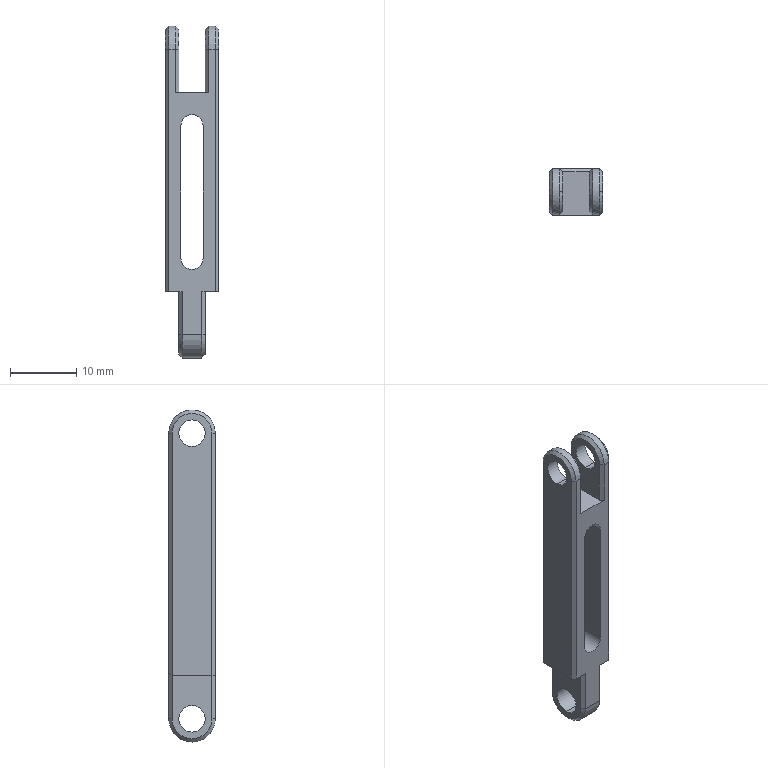Part | SolidWorks | features ICE 3, Chamfer 1, Extrusion 1, Scale 1 | 1 solid | 55 faces | box 8 x 7 x 50 mm | volume 1532 mm3 | plane 30 | cylinder 13 | cone 12 | commonest cylinder face diameters 4 x6 7 x4 3.32 x3
STEP:
#1=CARTESIAN_POINT('',(0.,6.5,6.66));
#2=VERTEX_POINT('',#1);
#3=CARTESIAN_POINT('',(1.66,6.5,5.));
#4=VERTEX_POINT('',#3);
#5=CARTESIAN_POINT('',(0.,6.5,5.));
#6=DIRECTION('',(0.,1.,0.));
#7=DIRECTION('',(0.,0.,-1.));
#8=AXIS2_PLACEMENT_3D('',#5,#6,#7);
#9=CIRCLE('',#8,1.66);
#10=EDGE_CURVE('',#2,#4,#9,.T.);
#11=ORIENTED_EDGE('',*,*,#10,.F.);
#12=CARTESIAN_POINT('',(0.,7.,7.16));
#13=VERTEX_POINT('',#12);
#14=CARTESIAN_POINT('',(0.,6.5,6.66));
#15=DIRECTION('',(0.,0.7071,0.7071));
#16=VECTOR('',#15,1000.);
#17=LINE('',#14,#16);
#18=EDGE_CURVE('',#2,#13,#17,.T.);
#19=ORIENTED_EDGE('',*,*,#18,.T.);
#20=CARTESIAN_POINT('',(2.16,7.,5.));
#21=VERTEX_POINT('',#20);
#22=CARTESIAN_POINT('',(0.,7.,5.));
#23=DIRECTION('',(0.,-1.,0.));
#24=DIRECTION('',(0.,0.,-1.));
#25=AXIS2_PLACEMENT_3D('',#22,#23,#24);
#26=CIRCLE('',#25,2.16);
#27=EDGE_CURVE('',#21,#13,#26,.T.);
#28=ORIENTED_EDGE('',*,*,#27,.F.);
#29=CARTESIAN_POINT('',(2.16,7.,5.));
#30=DIRECTION('',(-0.7071,-0.7071,0.));
#31=VECTOR('',#30,1000.);
#32=LINE('',#29,#31);
#33=EDGE_CURVE('',#21,#4,#32,.T.);
#34=ORIENTED_EDGE('',*,*,#33,.T.);
#35=EDGE_LOOP('',(#11,#19,#28,#34));
#36=FACE_OUTER_BOUND('',#35,.T.);
#37=CARTESIAN_POINT('',(0.,6.5,5.));
#38=DIRECTION('',(0.,1.,0.));
#39=DIRECTION('',(0.,0.,1.));
#40=AXIS2_PLACEMENT_3D('',#37,#38,#39);
#41=CONICAL_SURFACE('',#40,1.66,0.7854);
#42=ADVANCED_FACE('',(#36),#41,.F.);
#43=CARTESIAN_POINT('',(-2.,3.5,-29.5));
#44=VERTEX_POINT('',#43);
#45=CARTESIAN_POINT('',(-2.,0.5,-26.5));
#46=VERTEX_POINT('',#45);
#47=CARTESIAN_POINT('',(-2.,3.5,-26.5));
#48=DIRECTION('',(-1.,0.,0.));
#49=DIRECTION('',(0.,0.,-1.));
#50=AXIS2_PLACEMENT_3D('',#47,#48,#49);
#51=CIRCLE('',#50,3.);
#52=EDGE_CURVE('',#44,#46,#51,.T.);
#53=ORIENTED_EDGE('',*,*,#52,.F.);
#54=CARTESIAN_POINT('',(-1.5,3.5,-30.));
#55=VERTEX_POINT('',#54);
#56=CARTESIAN_POINT('',(-1.5,3.5,-30.));
#57=DIRECTION('',(0.7071,0.,-0.7071));
#58=VECTOR('',#57,1000.);
#59=LINE('',#56,#58);
#60=EDGE_CURVE('',#44,#55,#59,.T.);
#61=ORIENTED_EDGE('',*,*,#60,.T.);
#62=CARTESIAN_POINT('',(-1.5,0.,-26.5));
#63=VERTEX_POINT('',#62);
#64=CARTESIAN_POINT('',(-1.5,3.5,-26.5));
#65=DIRECTION('',(1.,0.,0.));
#66=DIRECTION('',(0.,0.,-1.));
#67=AXIS2_PLACEMENT_3D('',#64,#65,#66);
#68=CIRCLE('',#67,3.5);
#69=EDGE_CURVE('',#63,#55,#68,.T.);
#70=ORIENTED_EDGE('',*,*,#69,.F.);
#71=CARTESIAN_POINT('',(-2.,0.5,-26.5));
#72=DIRECTION('',(0.7071,-0.7071,0.));
#73=VECTOR('',#72,1000.);
#74=LINE('',#71,#73);
#75=EDGE_CURVE('',#46,#63,#74,.T.);
#76=ORIENTED_EDGE('',*,*,#75,.F.);
#77=EDGE_LOOP('',(#53,#61,#70,#76));
#78=FACE_OUTER_BOUND('',#77,.T.);
#79=CARTESIAN_POINT('',(-1.5,3.5,-26.5));
#80=DIRECTION('',(1.,0.,0.));
#81=DIRECTION('',(0.,0.,-1.));
#82=AXIS2_PLACEMENT_3D('',#79,#80,#81);
#83=CONICAL_SURFACE('',#82,3.5,0.7854);
#84=ADVANCED_FACE('',(#78),#83,.T.);
#85=CARTESIAN_POINT('',(-2.,3.5,19.5));
#86=VERTEX_POINT('',#85);
#87=CARTESIAN_POINT('',(-2.,0.5,16.5));
#88=VERTEX_POINT('',#87);
#89=CARTESIAN_POINT('',(-2.,3.5,16.5));
#90=DIRECTION('',(1.,0.,0.));
#91=DIRECTION('',(0.,0.,1.));
#92=AXIS2_PLACEMENT_3D('',#89,#90,#91);
#93=CIRCLE('',#92,3.);
#94=EDGE_CURVE('',#86,#88,#93,.T.);
#95=ORIENTED_EDGE('',*,*,#94,.F.);
#96=CARTESIAN_POINT('',(-2.5,3.5,20.));
#97=VERTEX_POINT('',#96);
#98=CARTESIAN_POINT('',(-2.5,3.5,20.));
#99=DIRECTION('',(-0.7071,0.,0.7071));
#100=VECTOR('',#99,1000.);
#101=LINE('',#98,#100);
#102=EDGE_CURVE('',#86,#97,#101,.T.);
#103=ORIENTED_EDGE('',*,*,#102,.T.);
#104=CARTESIAN_POINT('',(-2.5,0.,16.5));
#105=VERTEX_POINT('',#104);
#106=CARTESIAN_POINT('',(-2.5,3.5,16.5));
#107=DIRECTION('',(-1.,0.,0.));
#108=DIRECTION('',(0.,0.,1.));
#109=AXIS2_PLACEMENT_3D('',#106,#107,#108);
#110=CIRCLE('',#109,3.5);
#111=EDGE_CURVE('',#105,#97,#110,.T.);
#112=ORIENTED_EDGE('',*,*,#111,.F.);
#113=CARTESIAN_POINT('',(-2.5,0.,16.5));
#114=DIRECTION('',(0.7071,0.7071,0.));
#115=VECTOR('',#114,1000.);
#116=LINE('',#113,#115);
#117=EDGE_CURVE('',#105,#88,#116,.T.);
#118=ORIENTED_EDGE('',*,*,#117,.T.);
#119=EDGE_LOOP('',(#95,#103,#112,#118));
#120=FACE_OUTER_BOUND('',#119,.T.);
#121=CARTESIAN_POINT('',(-2.5,3.5,16.5));
#122=DIRECTION('',(-1.,0.,0.));
#123=DIRECTION('',(0.,0.,1.));
#124=AXIS2_PLACEMENT_3D('',#121,#122,#123);
#125=CONICAL_SURFACE('',#124,3.5,0.7854);
#126=ADVANCED_FACE('',(#120),#125,.T.);
#127=CARTESIAN_POINT('',(4.,3.5,19.5));
#128=VERTEX_POINT('',#127);
#129=CARTESIAN_POINT('',(4.,0.5,16.5));
#130=VERTEX_POINT('',#129);
#131=CARTESIAN_POINT('',(4.,3.5,16.5));
#132=DIRECTION('',(1.,0.,0.));
#133=DIRECTION('',(0.,0.,1.));
#134=AXIS2_PLACEMENT_3D('',#131,#132,#133);
#135=CIRCLE('',#134,3.);
#136=EDGE_CURVE('',#128,#130,#135,.T.);
#137=ORIENTED_EDGE('',*,*,#136,.F.);
#138=CARTESIAN_POINT('',(3.5,3.5,20.));
#139=VERTEX_POINT('',#138);
#140=CARTESIAN_POINT('',(4.,3.5,19.5));
#141=DIRECTION('',(-0.7071,0.,0.7071));
#142=VECTOR('',#141,1000.);
#143=LINE('',#140,#142);
#144=EDGE_CURVE('',#128,#139,#143,.T.);
#145=ORIENTED_EDGE('',*,*,#144,.T.);
#146=CARTESIAN_POINT('',(3.5,0.,16.5));
#147=VERTEX_POINT('',#146);
#148=CARTESIAN_POINT('',(3.5,3.5,16.5));
#149=DIRECTION('',(-1.,0.,0.));
#150=DIRECTION('',(0.,0.,1.));
#151=AXIS2_PLACEMENT_3D('',#148,#149,#150);
#152=CIRCLE('',#151,3.5);
#153=EDGE_CURVE('',#147,#139,#152,.T.);
#154=ORIENTED_EDGE('',*,*,#153,.F.);
#155=CARTESIAN_POINT('',(3.5,0.,16.5));
#156=DIRECTION('',(0.7071,0.7071,0.));
#157=VECTOR('',#156,1000.);
#158=LINE('',#155,#157);
#159=EDGE_CURVE('',#147,#130,#158,.T.);
#160=ORIENTED_EDGE('',*,*,#159,.T.);
#161=EDGE_LOOP('',(#137,#145,#154,#160));
#162=FACE_OUTER_BOUND('',#161,.T.);
#163=CARTESIAN_POINT('',(4.,3.5,16.5));
#164=DIRECTION('',(-1.,0.,0.));
#165=DIRECTION('',(0.,0.,1.));
#166=AXIS2_PLACEMENT_3D('',#163,#164,#165);
#167=CONICAL_SURFACE('',#166,3.,0.7854);
#168=ADVANCED_FACE('',(#162),#167,.T.);
#169=CARTESIAN_POINT('',(0.,0.,6.66));
#170=VERTEX_POINT('',#169);
#171=CARTESIAN_POINT('',(1.66,0.,5.));
#172=VERTEX_POINT('',#171);
#173=CARTESIAN_POINT('',(0.,0.,5.));
#174=DIRECTION('',(0.,1.,0.));
#175=DIRECTION('',(0.,0.,1.));
#176=AXIS2_PLACEMENT_3D('',#173,#174,#175);
#177=CIRCLE('',#176,1.66);
#178=EDGE_CURVE('',#170,#172,#177,.T.);
#179=ORIENTED_EDGE('',*,*,#178,.F.);
#180=CARTESIAN_POINT('',(0.,0.,6.66));
#181=DIRECTION('',(0.,1.,0.));
#182=VECTOR('',#181,1000.);
#183=LINE('',#180,#182);
#184=EDGE_CURVE('',#170,#2,#183,.T.);
#185=ORIENTED_EDGE('',*,*,#184,.T.);
#186=ORIENTED_EDGE('',*,*,#10,.T.);
#187=CARTESIAN_POINT('',(1.66,0.,5.));
#188=DIRECTION('',(0.,1.,0.));
#189=VECTOR('',#188,1000.);
#190=LINE('',#187,#189);
#191=EDGE_CURVE('',#172,#4,#190,.T.);
#192=ORIENTED_EDGE('',*,*,#191,.F.);
#193=EDGE_LOOP('',(#179,#185,#186,#192));
#194=FACE_OUTER_BOUND('',#193,.T.);
#195=CARTESIAN_POINT('',(0.,0.,5.));
#196=DIRECTION('',(0.,1.,0.));
#197=DIRECTION('',(0.,0.,1.));
#198=AXIS2_PLACEMENT_3D('',#195,#196,#197);
#199=CYLINDRICAL_SURFACE('',#198,1.66);
#200=ADVANCED_FACE('',(#194),#199,.F.);
#201=CARTESIAN_POINT('',(-4.,3.5,18.5));
#202=VERTEX_POINT('',#201);
#203=CARTESIAN_POINT('',(-4.,3.5,14.5));
#204=VERTEX_POINT('',#203);
#205=CARTESIAN_POINT('',(-4.,3.5,16.5));
#206=DIRECTION('',(1.,0.,0.));
#207=DIRECTION('',(0.,0.,-1.));
#208=AXIS2_PLACEMENT_3D('',#205,#206,#207);
#209=CIRCLE('',#208,2.);
#210=EDGE_CURVE('',#202,#204,#209,.T.);
#211=ORIENTED_EDGE('',*,*,#210,.F.);
#212=CARTESIAN_POINT('',(-2.,3.5,18.5));
#213=VERTEX_POINT('',#212);
#214=CARTESIAN_POINT('',(-11.,3.5,18.5));
#215=DIRECTION('',(1.,0.,0.));
#216=VECTOR('',#215,1000.);
#217=LINE('',#214,#216);
#218=EDGE_CURVE('',#202,#213,#217,.T.);
#219=ORIENTED_EDGE('',*,*,#218,.T.);
#220=CARTESIAN_POINT('',(-2.,3.5,14.5));
#221=VERTEX_POINT('',#220);
#222=CARTESIAN_POINT('',(-2.,3.5,16.5));
#223=DIRECTION('',(-1.,0.,0.));
#224=DIRECTION('',(0.,0.,1.));
#225=AXIS2_PLACEMENT_3D('',#222,#223,#224);
#226=CIRCLE('',#225,2.);
#227=EDGE_CURVE('',#221,#213,#226,.T.);
#228=ORIENTED_EDGE('',*,*,#227,.F.);
#229=CARTESIAN_POINT('',(-11.,3.5,14.5));
#230=DIRECTION('',(1.,0.,0.));
#231=VECTOR('',#230,1000.);
#232=LINE('',#229,#231);
#233=EDGE_CURVE('',#204,#221,#232,.T.);
#234=ORIENTED_EDGE('',*,*,#233,.F.);
#235=EDGE_LOOP('',(#211,#219,#228,#234));
#236=FACE_OUTER_BOUND('',#235,.T.);
#237=CARTESIAN_POINT('',(-11.,3.5,16.5));
#238=DIRECTION('',(1.,0.,0.));
#239=DIRECTION('',(0.,0.,-1.));
#240=AXIS2_PLACEMENT_3D('',#237,#238,#239);
#241=CYLINDRICAL_SURFACE('',#240,2.);
#242=ADVANCED_FACE('',(#236),#241,.F.);
#243=CARTESIAN_POINT('',(2.,3.5,18.5));
#244=VERTEX_POINT('',#243);
#245=CARTESIAN_POINT('',(2.,3.5,14.5));
#246=VERTEX_POINT('',#245);
#247=CARTESIAN_POINT('',(2.,3.5,16.5));
#248=DIRECTION('',(1.,0.,0.));
#249=DIRECTION('',(0.,0.,-1.));
#250=AXIS2_PLACEMENT_3D('',#247,#248,#249);
#251=CIRCLE('',#250,2.);
#252=EDGE_CURVE('',#244,#246,#251,.T.);
#253=ORIENTED_EDGE('',*,*,#252,.F.);
#254=CARTESIAN_POINT('',(4.,3.5,18.5));
#255=VERTEX_POINT('',#254);
#256=CARTESIAN_POINT('',(-11.,3.5,18.5));
#257=DIRECTION('',(1.,0.,0.));
#258=VECTOR('',#257,1000.);
#259=LINE('',#256,#258);
#260=EDGE_CURVE('',#244,#255,#259,.T.);
#261=ORIENTED_EDGE('',*,*,#260,.T.);
#262=CARTESIAN_POINT('',(4.,3.5,14.5));
#263=VERTEX_POINT('',#262);
#264=CARTESIAN_POINT('',(4.,3.5,16.5));
#265=DIRECTION('',(1.,0.,0.));
#266=DIRECTION('',(0.,0.,-1.));
#267=AXIS2_PLACEMENT_3D('',#264,#265,#266);
#268=CIRCLE('',#267,2.);
#269=EDGE_CURVE('',#255,#263,#268,.T.);
#270=ORIENTED_EDGE('',*,*,#269,.T.);
#271=CARTESIAN_POINT('',(-11.,3.5,14.5));
#272=DIRECTION('',(1.,0.,0.));
#273=VECTOR('',#272,1000.);
#274=LINE('',#271,#273);
#275=EDGE_CURVE('',#246,#263,#274,.T.);
#276=ORIENTED_EDGE('',*,*,#275,.F.);
#277=EDGE_LOOP('',(#253,#261,#270,#276));
#278=FACE_OUTER_BOUND('',#277,.T.);
#279=CARTESIAN_POINT('',(-11.,3.5,16.5));
#280=DIRECTION('',(1.,0.,0.));
#281=DIRECTION('',(0.,0.,-1.));
#282=AXIS2_PLACEMENT_3D('',#279,#280,#281);
#283=CYLINDRICAL_SURFACE('',#282,2.);
#284=ADVANCED_FACE('',(#278),#283,.F.);
#285=CARTESIAN_POINT('',(-2.,3.5,-24.5));
#286=VERTEX_POINT('',#285);
#287=CARTESIAN_POINT('',(-2.,3.5,-28.5));
#288=VERTEX_POINT('',#287);
#289=CARTESIAN_POINT('',(-2.,3.5,-26.5));
#290=DIRECTION('',(1.,0.,0.));
#291=DIRECTION('',(0.,0.,-1.));
#292=AXIS2_PLACEMENT_3D('',#289,#290,#291);
#293=CIRCLE('',#292,2.);
#294=EDGE_CURVE('',#286,#288,#293,.T.);
#295=ORIENTED_EDGE('',*,*,#294,.F.);
#296=CARTESIAN_POINT('',(2.,3.5,-24.5));
#297=VERTEX_POINT('',#296);
#298=CARTESIAN_POINT('',(-5.,3.5,-24.5));
#299=DIRECTION('',(1.,0.,0.));
#300=VECTOR('',#299,1000.);
#301=LINE('',#298,#300);
#302=EDGE_CURVE('',#286,#297,#301,.T.);
#303=ORIENTED_EDGE('',*,*,#302,.T.);
#304=CARTESIAN_POINT('',(2.,3.5,-28.5));
#305=VERTEX_POINT('',#304);
#306=CARTESIAN_POINT('',(2.,3.5,-26.5));
#307=DIRECTION('',(1.,0.,0.));
#308=DIRECTION('',(0.,0.,-1.));
#309=AXIS2_PLACEMENT_3D('',#306,#307,#308);
#310=CIRCLE('',#309,2.);
#311=EDGE_CURVE('',#297,#305,#310,.T.);
#312=ORIENTED_EDGE('',*,*,#311,.T.);
#313=CARTESIAN_POINT('',(-5.,3.5,-28.5));
#314=DIRECTION('',(1.,0.,0.));
#315=VECTOR('',#314,1000.);
#316=LINE('',#313,#315);
#317=EDGE_CURVE('',#288,#305,#316,.T.);
#318=ORIENTED_EDGE('',*,*,#317,.F.);
#319=EDGE_LOOP('',(#295,#303,#312,#318));
#320=FACE_OUTER_BOUND('',#319,.T.);
#321=CARTESIAN_POINT('',(-5.,3.5,-26.5));
#322=DIRECTION('',(1.,0.,0.));
#323=DIRECTION('',(0.,0.,-1.));
#324=AXIS2_PLACEMENT_3D('',#321,#322,#323);
#325=CYLINDRICAL_SURFACE('',#324,2.);
#326=ADVANCED_FACE('',(#320),#325,.F.);
#327=ORIENTED_EDGE('',*,*,#69,.T.);
#328=CARTESIAN_POINT('',(1.5,3.5,-30.));
#329=VERTEX_POINT('',#328);
#330=CARTESIAN_POINT('',(-5.,3.5,-30.));
#331=DIRECTION('',(1.,0.,0.));
#332=VECTOR('',#331,1000.);
#333=LINE('',#330,#332);
#334=EDGE_CURVE('',#55,#329,#333,.T.);
#335=ORIENTED_EDGE('',*,*,#334,.T.);
#336=CARTESIAN_POINT('',(1.5,0.,-26.5));
#337=VERTEX_POINT('',#336);
#338=CARTESIAN_POINT('',(1.5,3.5,-26.5));
#339=DIRECTION('',(-1.,0.,0.));
#340=DIRECTION('',(0.,0.,1.));
#341=AXIS2_PLACEMENT_3D('',#338,#339,#340);
#342=CIRCLE('',#341,3.5);
#343=EDGE_CURVE('',#329,#337,#342,.T.);
#344=ORIENTED_EDGE('',*,*,#343,.T.);
#345=CARTESIAN_POINT('',(-5.,0.,-26.5));
#346=DIRECTION('',(1.,0.,0.));
#347=VECTOR('',#346,1000.);
#348=LINE('',#345,#347);
#349=EDGE_CURVE('',#63,#337,#348,.T.);
#350=ORIENTED_EDGE('',*,*,#349,.F.);
#351=EDGE_LOOP('',(#327,#335,#344,#350));
#352=FACE_OUTER_BOUND('',#351,.T.);
#353=CARTESIAN_POINT('',(-5.,3.5,-26.5));
#354=DIRECTION('',(1.,0.,0.));
#355=DIRECTION('',(0.,0.,-1.));
#356=AXIS2_PLACEMENT_3D('',#353,#354,#355);
#357=CYLINDRICAL_SURFACE('',#356,3.5);
#358=ADVANCED_FACE('',(#352),#357,.T.);
#359=CARTESIAN_POINT('',(4.,3.5,16.5));
#360=DIRECTION('',(1.,0.,0.));
#361=DIRECTION('',(0.,0.,-1.));
#362=AXIS2_PLACEMENT_3D('',#359,#360,#361);
#363=CIRCLE('',#362,2.);
#364=EDGE_CURVE('',#263,#255,#363,.T.);
#365=ORIENTED_EDGE('',*,*,#364,.F.);
#366=ORIENTED_EDGE('',*,*,#269,.F.);
#367=EDGE_LOOP('',(#365,#366));
#368=FACE_BOUND('',#367,.T.);
#369=CARTESIAN_POINT('',(4.,6.5,16.5));
#370=VERTEX_POINT('',#369);
#371=CARTESIAN_POINT('',(4.,3.5,16.5));
#372=DIRECTION('',(1.,0.,0.));
#373=DIRECTION('',(0.,0.,1.));
#374=AXIS2_PLACEMENT_3D('',#371,#372,#373);
#375=CIRCLE('',#374,3.);
#376=EDGE_CURVE('',#370,#128,#375,.T.);
#377=ORIENTED_EDGE('',*,*,#376,.T.);
#378=ORIENTED_EDGE('',*,*,#136,.T.);
#379=CARTESIAN_POINT('',(4.,0.5,-20.));
#380=VERTEX_POINT('',#379);
#381=CARTESIAN_POINT('',(4.,0.5,-20.));
#382=DIRECTION('',(0.,0.,-1.));
#383=VECTOR('',#382,1000.);
#384=LINE('',#381,#383);
#385=EDGE_CURVE('',#130,#380,#384,.T.);
#386=ORIENTED_EDGE('',*,*,#385,.T.);
#387=CARTESIAN_POINT('',(4.,6.5,-20.));
#388=VERTEX_POINT('',#387);
#389=CARTESIAN_POINT('',(4.,7.,-20.));
#390=DIRECTION('',(0.,-1.,0.));
#391=VECTOR('',#390,1000.);
#392=LINE('',#389,#391);
#393=EDGE_CURVE('',#388,#380,#392,.T.);
#394=ORIENTED_EDGE('',*,*,#393,.F.);
#395=CARTESIAN_POINT('',(4.,6.5,-20.));
#396=DIRECTION('',(0.,0.,1.));
#397=VECTOR('',#396,1000.);
#398=LINE('',#395,#397);
#399=EDGE_CURVE('',#388,#370,#398,.T.);
#400=ORIENTED_EDGE('',*,*,#399,.T.);
#401=EDGE_LOOP('',(#377,#378,#386,#394,#400));
#402=FACE_OUTER_BOUND('',#401,.T.);
#403=CARTESIAN_POINT('',(4.,7.,-20.));
#404=DIRECTION('',(-1.,0.,0.));
#405=DIRECTION('',(0.,0.,1.));
#406=AXIS2_PLACEMENT_3D('',#403,#404,#405);
#407=PLANE('',#406);
#408=ADVANCED_FACE('',(#368,#402),#407,.F.);
#409=CARTESIAN_POINT('',(-4.,3.5,16.5));
#410=DIRECTION('',(1.,0.,0.));
#411=DIRECTION('',(0.,0.,-1.));
#412=AXIS2_PLACEMENT_3D('',#409,#410,#411);
#413=CIRCLE('',#412,2.);
#414=EDGE_CURVE('',#204,#202,#413,.T.);
#415=ORIENTED_EDGE('',*,*,#414,.T.);
#416=ORIENTED_EDGE('',*,*,#210,.T.);
#417=EDGE_LOOP('',(#415,#416));
#418=FACE_BOUND('',#417,.T.);
#419=CARTESIAN_POINT('',(-4.,6.5,-20.));
#420=VERTEX_POINT('',#419);
#421=CARTESIAN_POINT('',(-4.,0.5,-20.));
#422=VERTEX_POINT('',#421);
#423=CARTESIAN_POINT('',(-4.,7.,-20.));
#424=DIRECTION('',(0.,-1.,0.));
#425=VECTOR('',#424,1000.);
#426=LINE('',#423,#425);
#427=EDGE_CURVE('',#420,#422,#426,.T.);
#428=ORIENTED_EDGE('',*,*,#427,.T.);
#429=CARTESIAN_POINT('',(-4.,0.5,16.5));
#430=VERTEX_POINT('',#429);
#431=CARTESIAN_POINT('',(-4.,0.5,16.5));
#432=DIRECTION('',(0.,0.,1.));
#433=VECTOR('',#432,1000.);
#434=LINE('',#431,#433);
#435=EDGE_CURVE('',#422,#430,#434,.T.);
#436=ORIENTED_EDGE('',*,*,#435,.T.);
#437=CARTESIAN_POINT('',(-4.,6.5,16.5));
#438=VERTEX_POINT('',#437);
#439=CARTESIAN_POINT('',(-4.,3.5,16.5));
#440=DIRECTION('',(-1.,0.,0.));
#441=DIRECTION('',(0.,0.,-1.));
#442=AXIS2_PLACEMENT_3D('',#439,#440,#441);
#443=CIRCLE('',#442,3.);
#444=EDGE_CURVE('',#430,#438,#443,.T.);
#445=ORIENTED_EDGE('',*,*,#444,.T.);
#446=CARTESIAN_POINT('',(-4.,6.5,-20.));
#447=DIRECTION('',(0.,0.,-1.));
#448=VECTOR('',#447,1000.);
#449=LINE('',#446,#448);
#450=EDGE_CURVE('',#438,#420,#449,.T.);
#451=ORIENTED_EDGE('',*,*,#450,.T.);
#452=EDGE_LOOP('',(#428,#436,#445,#451));
#453=FACE_OUTER_BOUND('',#452,.T.);
#454=CARTESIAN_POINT('',(-4.,7.,-20.));
#455=DIRECTION('',(1.,0.,0.));
#456=DIRECTION('',(0.,0.,-1.));
#457=AXIS2_PLACEMENT_3D('',#454,#455,#456);
#458=PLANE('',#457);
#459=ADVANCED_FACE('',(#418,#453),#458,.F.);
#460=ORIENTED_EDGE('',*,*,#227,.T.);
#461=CARTESIAN_POINT('',(-2.,3.5,16.5));
#462=DIRECTION('',(-1.,0.,0.));
#463=DIRECTION('',(0.,0.,1.));
#464=AXIS2_PLACEMENT_3D('',#461,#462,#463);
#465=CIRCLE('',#464,2.);
#466=EDGE_CURVE('',#213,#221,#465,.T.);
#467=ORIENTED_EDGE('',*,*,#466,.T.);
#468=EDGE_LOOP('',(#460,#467));
#469=FACE_BOUND('',#468,.T.);
#470=CARTESIAN_POINT('',(-2.,6.5,16.5));
#471=VERTEX_POINT('',#470);
#472=CARTESIAN_POINT('',(-2.,3.5,16.5));
#473=DIRECTION('',(1.,0.,0.));
#474=DIRECTION('',(0.,0.,1.));
#475=AXIS2_PLACEMENT_3D('',#472,#473,#474);
#476=CIRCLE('',#475,3.);
#477=EDGE_CURVE('',#471,#86,#476,.T.);
#478=ORIENTED_EDGE('',*,*,#477,.T.);
#479=ORIENTED_EDGE('',*,*,#94,.T.);
#480=CARTESIAN_POINT('',(-2.,0.5,10.));
#481=VERTEX_POINT('',#480);
#482=CARTESIAN_POINT('',(-2.,0.5,10.));
#483=DIRECTION('',(0.,0.,-1.));
#484=VECTOR('',#483,1000.);
#485=LINE('',#482,#484);
#486=EDGE_CURVE('',#88,#481,#485,.T.);
#487=ORIENTED_EDGE('',*,*,#486,.T.);
#488=CARTESIAN_POINT('',(-2.,6.5,10.));
#489=VERTEX_POINT('',#488);
#490=CARTESIAN_POINT('',(-2.,7.,10.));
#491=DIRECTION('',(0.,-1.,0.));
#492=VECTOR('',#491,1000.);
#493=LINE('',#490,#492);
#494=EDGE_CURVE('',#489,#481,#493,.T.);
#495=ORIENTED_EDGE('',*,*,#494,.F.);
#496=CARTESIAN_POINT('',(-2.,6.5,20.));
#497=DIRECTION('',(0.,0.,1.));
#498=VECTOR('',#497,1000.);
#499=LINE('',#496,#498);
#500=EDGE_CURVE('',#489,#471,#499,.T.);
#501=ORIENTED_EDGE('',*,*,#500,.T.);
#502=EDGE_LOOP('',(#478,#479,#487,#495,#501));
#503=FACE_OUTER_BOUND('',#502,.T.);
#504=CARTESIAN_POINT('',(-2.,7.,20.));
#505=DIRECTION('',(-1.,0.,0.));
#506=DIRECTION('',(0.,0.,1.));
#507=AXIS2_PLACEMENT_3D('',#504,#505,#506);
#508=PLANE('',#507);
#509=ADVANCED_FACE('',(#469,#503),#508,.F.);
#510=CARTESIAN_POINT('',(2.,3.5,16.5));
#511=DIRECTION('',(1.,0.,0.));
#512=DIRECTION('',(0.,0.,-1.));
#513=AXIS2_PLACEMENT_3D('',#510,#511,#512);
#514=CIRCLE('',#513,2.);
#515=EDGE_CURVE('',#246,#244,#514,.T.);
#516=ORIENTED_EDGE('',*,*,#515,.T.);
#517=ORIENTED_EDGE('',*,*,#252,.T.);
#518=EDGE_LOOP('',(#516,#517));
#519=FACE_BOUND('',#518,.T.);
#520=CARTESIAN_POINT('',(2.,6.5,10.));
#521=VERTEX_POINT('',#520);
#522=CARTESIAN_POINT('',(2.,0.5,10.));
#523=VERTEX_POINT('',#522);
#524=CARTESIAN_POINT('',(2.,7.,10.));
#525=DIRECTION('',(0.,-1.,0.));
#526=VECTOR('',#525,1000.);
#527=LINE('',#524,#526);
#528=EDGE_CURVE('',#521,#523,#527,.T.);
#529=ORIENTED_EDGE('',*,*,#528,.T.);
#530=CARTESIAN_POINT('',(2.,0.5,16.5));
#531=VERTEX_POINT('',#530);
#532=CARTESIAN_POINT('',(2.,0.5,16.5));
#533=DIRECTION('',(0.,0.,1.));
#534=VECTOR('',#533,1000.);
#535=LINE('',#532,#534);
#536=EDGE_CURVE('',#523,#531,#535,.T.);
#537=ORIENTED_EDGE('',*,*,#536,.T.);
#538=CARTESIAN_POINT('',(2.,6.5,16.5));
#539=VERTEX_POINT('',#538);
#540=CARTESIAN_POINT('',(2.,3.5,16.5));
#541=DIRECTION('',(-1.,0.,0.));
#542=DIRECTION('',(0.,0.,-1.));
#543=AXIS2_PLACEMENT_3D('',#540,#541,#542);
#544=CIRCLE('',#543,3.);
#545=EDGE_CURVE('',#531,#539,#544,.T.);
#546=ORIENTED_EDGE('',*,*,#545,.T.);
#547=CARTESIAN_POINT('',(2.,6.5,20.));
#548=DIRECTION('',(0.,0.,-1.));
#549=VECTOR('',#548,1000.);
#550=LINE('',#547,#549);
#551=EDGE_CURVE('',#539,#521,#550,.T.);
#552=ORIENTED_EDGE('',*,*,#551,.T.);
#553=EDGE_LOOP('',(#529,#537,#546,#552));
#554=FACE_OUTER_BOUND('',#553,.T.);
#555=CARTESIAN_POINT('',(2.,7.,20.));
#556=DIRECTION('',(1.,0.,0.));
#557=DIRECTION('',(0.,0.,-1.));
#558=AXIS2_PLACEMENT_3D('',#555,#556,#557);
#559=PLANE('',#558);
#560=ADVANCED_FACE('',(#519,#554),#559,.F.);
#561=CARTESIAN_POINT('',(2.,3.5,-26.5));
#562=DIRECTION('',(1.,0.,0.));
#563=DIRECTION('',(0.,0.,-1.));
#564=AXIS2_PLACEMENT_3D('',#561,#562,#563);
#565=CIRCLE('',#564,2.);
#566=EDGE_CURVE('',#305,#297,#565,.T.);
#567=ORIENTED_EDGE('',*,*,#566,.F.);
#568=ORIENTED_EDGE('',*,*,#311,.F.);
#569=EDGE_LOOP('',(#567,#568));
#570=FACE_BOUND('',#569,.T.);
#571=CARTESIAN_POINT('',(2.,6.5,-20.));
#572=VERTEX_POINT('',#571);
#573=CARTESIAN_POINT('',(2.,0.5,-20.));
#574=VERTEX_POINT('',#573);
#575=CARTESIAN_POINT('',(2.,7.,-20.));
#576=DIRECTION('',(0.,-1.,0.));
#577=VECTOR('',#576,1000.);
#578=LINE('',#575,#577);
#579=EDGE_CURVE('',#572,#574,#578,.T.);
#580=ORIENTED_EDGE('',*,*,#579,.T.);
#581=CARTESIAN_POINT('',(2.,0.5,-26.5));
#582=VERTEX_POINT('',#581);
#583=CARTESIAN_POINT('',(2.,0.5,-26.5));
#584=DIRECTION('',(0.,0.,-1.));
#585=VECTOR('',#584,1000.);
#586=LINE('',#583,#585);
#587=EDGE_CURVE('',#574,#582,#586,.T.);
#588=ORIENTED_EDGE('',*,*,#587,.T.);
#589=CARTESIAN_POINT('',(2.,6.5,-26.5));
#590=VERTEX_POINT('',#589);
#591=CARTESIAN_POINT('',(2.,3.5,-26.5));
#592=DIRECTION('',(1.,0.,0.));
#593=DIRECTION('',(0.,0.,1.));
#594=AXIS2_PLACEMENT_3D('',#591,#592,#593);
#595=CIRCLE('',#594,3.);
#596=EDGE_CURVE('',#582,#590,#595,.T.);
#597=ORIENTED_EDGE('',*,*,#596,.T.);
#598=CARTESIAN_POINT('',(2.,6.5,-20.));
#599=DIRECTION('',(0.,0.,1.));
#600=VECTOR('',#599,1000.);
#601=LINE('',#598,#600);
#602=EDGE_CURVE('',#590,#572,#601,.T.);
#603=ORIENTED_EDGE('',*,*,#602,.T.);
#604=EDGE_LOOP('',(#580,#588,#597,#603));
#605=FACE_OUTER_BOUND('',#604,.T.);
#606=CARTESIAN_POINT('',(2.,7.,-20.));
#607=DIRECTION('',(-1.,0.,0.));
#608=DIRECTION('',(0.,0.,1.));
#609=AXIS2_PLACEMENT_3D('',#606,#607,#608);
#610=PLANE('',#609);
#611=ADVANCED_FACE('',(#570,#605),#610,.F.);
#612=CARTESIAN_POINT('',(-2.,3.5,-26.5));
#613=DIRECTION('',(1.,0.,0.));
#614=DIRECTION('',(0.,0.,-1.));
#615=AXIS2_PLACEMENT_3D('',#612,#613,#614);
#616=CIRCLE('',#615,2.);
#617=EDGE_CURVE('',#288,#286,#616,.T.);
#618=ORIENTED_EDGE('',*,*,#617,.T.);
#619=ORIENTED_EDGE('',*,*,#294,.T.);
#620=EDGE_LOOP('',(#618,#619));
#621=FACE_BOUND('',#620,.T.);
#622=CARTESIAN_POINT('',(-2.,6.5,-26.5));
#623=VERTEX_POINT('',#622);
#624=CARTESIAN_POINT('',(-2.,3.5,-26.5));
#625=DIRECTION('',(-1.,0.,0.));
#626=DIRECTION('',(0.,0.,-1.));
#627=AXIS2_PLACEMENT_3D('',#624,#625,#626);
#628=CIRCLE('',#627,3.);
#629=EDGE_CURVE('',#623,#44,#628,.T.);
#630=ORIENTED_EDGE('',*,*,#629,.T.);
#631=ORIENTED_EDGE('',*,*,#52,.T.);
#632=CARTESIAN_POINT('',(-2.,0.5,-20.));
#633=VERTEX_POINT('',#632);
#634=CARTESIAN_POINT('',(-2.,0.5,-20.));
#635=DIRECTION('',(0.,0.,1.));
#636=VECTOR('',#635,1000.);
#637=LINE('',#634,#636);
#638=EDGE_CURVE('',#46,#633,#637,.T.);
#639=ORIENTED_EDGE('',*,*,#638,.T.);
#640=CARTESIAN_POINT('',(-2.,6.5,-20.));
#641=VERTEX_POINT('',#640);
#642=CARTESIAN_POINT('',(-2.,7.,-20.));
#643=DIRECTION('',(0.,-1.,0.));
#644=VECTOR('',#643,1000.);
#645=LINE('',#642,#644);
#646=EDGE_CURVE('',#641,#633,#645,.T.);
#647=ORIENTED_EDGE('',*,*,#646,.F.);
#648=CARTESIAN_POINT('',(-2.,6.5,-20.));
#649=DIRECTION('',(0.,0.,-1.));
#650=VECTOR('',#649,1000.);
#651=LINE('',#648,#650);
#652=EDGE_CURVE('',#641,#623,#651,.T.);
#653=ORIENTED_EDGE('',*,*,#652,.T.);
#654=EDGE_LOOP('',(#630,#631,#639,#647,#653));
#655=FACE_OUTER_BOUND('',#654,.T.);
#656=CARTESIAN_POINT('',(-2.,7.,-20.));
#657=DIRECTION('',(1.,0.,0.));
#658=DIRECTION('',(0.,0.,-1.));
#659=AXIS2_PLACEMENT_3D('',#656,#657,#658);
#660=PLANE('',#659);
#661=ADVANCED_FACE('',(#621,#655),#660,.F.);
#662=CARTESIAN_POINT('',(1.66,0.,-15.));
#663=VERTEX_POINT('',#662);
#664=CARTESIAN_POINT('',(-1.66,0.,-15.));
#665=VERTEX_POINT('',#664);
#666=CARTESIAN_POINT('',(0.,0.,-15.));
#667=DIRECTION('',(0.,1.,0.));
#668=DIRECTION('',(0.,0.,1.));
#669=AXIS2_PLACEMENT_3D('',#666,#667,#668);
#670=CIRCLE('',#669,1.66);
#671=EDGE_CURVE('',#663,#665,#670,.T.);
#672=ORIENTED_EDGE('',*,*,#671,.T.);
#673=CARTESIAN_POINT('',(-1.66,0.,5.));
#674=VERTEX_POINT('',#673);
#675=CARTESIAN_POINT('',(-1.66,0.,-15.));
#676=DIRECTION('',(0.,0.,1.));
#677=VECTOR('',#676,1000.);
#678=LINE('',#675,#677);
#679=EDGE_CURVE('',#665,#674,#678,.T.);
#680=ORIENTED_EDGE('',*,*,#679,.T.);
#681=CARTESIAN_POINT('',(0.,0.,5.));
#682=DIRECTION('',(0.,1.,0.));
#683=DIRECTION('',(0.,0.,1.));
#684=AXIS2_PLACEMENT_3D('',#681,#682,#683);
#685=CIRCLE('',#684,1.66);
#686=EDGE_CURVE('',#674,#170,#685,.T.);
#687=ORIENTED_EDGE('',*,*,#686,.T.);
#688=ORIENTED_EDGE('',*,*,#178,.T.);
#689=CARTESIAN_POINT('',(1.66,0.,-15.));
#690=DIRECTION('',(0.,0.,-1.));
#691=VECTOR('',#690,1000.);
#692=LINE('',#689,#691);
#693=EDGE_CURVE('',#172,#663,#692,.T.);
#694=ORIENTED_EDGE('',*,*,#693,.T.);
#695=EDGE_LOOP('',(#672,#680,#687,#688,#694));
#696=FACE_BOUND('',#695,.T.);
#697=ORIENTED_EDGE('',*,*,#349,.T.);
#698=CARTESIAN_POINT('',(1.5,0.,-20.));
#699=VERTEX_POINT('',#698);
#700=CARTESIAN_POINT('',(1.5,0.,-20.));
#701=DIRECTION('',(0.,0.,1.));
#702=VECTOR('',#701,1000.);
#703=LINE('',#700,#702);
#704=EDGE_CURVE('',#337,#699,#703,.T.);
#705=ORIENTED_EDGE('',*,*,#704,.T.);
#706=CARTESIAN_POINT('',(3.5,0.,-20.));
#707=VERTEX_POINT('',#706);
#708=CARTESIAN_POINT('',(2.,0.,-20.));
#709=DIRECTION('',(-1.,0.,0.));
#710=VECTOR('',#709,1000.);
#711=LINE('',#708,#710);
#712=EDGE_CURVE('',#707,#699,#711,.T.);
#713=ORIENTED_EDGE('',*,*,#712,.F.);
#714=CARTESIAN_POINT('',(3.5,0.,16.5));
#715=DIRECTION('',(0.,0.,1.));
#716=VECTOR('',#715,1000.);
#717=LINE('',#714,#716);
#718=EDGE_CURVE('',#707,#147,#717,.T.);
#719=ORIENTED_EDGE('',*,*,#718,.T.);
#720=CARTESIAN_POINT('',(2.5,0.,16.5));
#721=VERTEX_POINT('',#720);
#722=CARTESIAN_POINT('',(-11.,0.,16.5));
#723=DIRECTION('',(1.,0.,0.));
#724=VECTOR('',#723,1000.);
#725=LINE('',#722,#724);
#726=EDGE_CURVE('',#721,#147,#725,.T.);
#727=ORIENTED_EDGE('',*,*,#726,.F.);
#728=CARTESIAN_POINT('',(2.5,0.,10.));
#729=VERTEX_POINT('',#728);
#730=CARTESIAN_POINT('',(2.5,0.,10.));
#731=DIRECTION('',(0.,0.,-1.));
#732=VECTOR('',#731,1000.);
#733=LINE('',#730,#732);
#734=EDGE_CURVE('',#721,#729,#733,.T.);
#735=ORIENTED_EDGE('',*,*,#734,.T.);
#736=CARTESIAN_POINT('',(-2.5,0.,10.));
#737=VERTEX_POINT('',#736);
#738=CARTESIAN_POINT('',(-2.,0.,10.));
#739=DIRECTION('',(1.,0.,0.));
#740=VECTOR('',#739,1000.);
#741=LINE('',#738,#740);
#742=EDGE_CURVE('',#737,#729,#741,.T.);
#743=ORIENTED_EDGE('',*,*,#742,.F.);
#744=CARTESIAN_POINT('',(-2.5,0.,16.5));
#745=DIRECTION('',(0.,0.,1.));
#746=VECTOR('',#745,1000.);
#747=LINE('',#744,#746);
#748=EDGE_CURVE('',#737,#105,#747,.T.);
#749=ORIENTED_EDGE('',*,*,#748,.T.);
#750=CARTESIAN_POINT('',(-3.5,0.,16.5));
#751=VERTEX_POINT('',#750);
#752=CARTESIAN_POINT('',(-11.,0.,16.5));
#753=DIRECTION('',(1.,0.,0.));
#754=VECTOR('',#753,1000.);
#755=LINE('',#752,#754);
#756=EDGE_CURVE('',#751,#105,#755,.T.);
#757=ORIENTED_EDGE('',*,*,#756,.F.);
#758=CARTESIAN_POINT('',(-3.5,0.,-20.));
#759=VERTEX_POINT('',#758);
#760=CARTESIAN_POINT('',(-3.5,0.,-20.));
#761=DIRECTION('',(0.,0.,-1.));
#762=VECTOR('',#761,1000.);
#763=LINE('',#760,#762);
#764=EDGE_CURVE('',#751,#759,#763,.T.);
#765=ORIENTED_EDGE('',*,*,#764,.T.);
#766=CARTESIAN_POINT('',(-1.5,0.,-20.));
#767=VERTEX_POINT('',#766);
#768=CARTESIAN_POINT('',(-4.,0.,-20.));
#769=DIRECTION('',(-1.,0.,0.));
#770=VECTOR('',#769,1000.);
#771=LINE('',#768,#770);
#772=EDGE_CURVE('',#767,#759,#771,.T.);
#773=ORIENTED_EDGE('',*,*,#772,.F.);
#774=CARTESIAN_POINT('',(-1.5,0.,-26.5));
#775=DIRECTION('',(0.,0.,-1.));
#776=VECTOR('',#775,1000.);
#777=LINE('',#774,#776);
#778=EDGE_CURVE('',#767,#63,#777,.T.);
#779=ORIENTED_EDGE('',*,*,#778,.T.);
#780=EDGE_LOOP('',(#697,#705,#713,#719,#727,#735,#743,#749,#757,#765,#773,#779));
#781=FACE_OUTER_BOUND('',#780,.T.);
#782=CARTESIAN_POINT('',(0.,0.,0.));
#783=DIRECTION('',(0.,-1.,0.));
#784=DIRECTION('',(0.,0.,-1.));
#785=AXIS2_PLACEMENT_3D('',#782,#783,#784);
#786=PLANE('',#785);
#787=ADVANCED_FACE('',(#696,#781),#786,.T.);
#788=CARTESIAN_POINT('',(2.16,7.,-15.));
#789=VERTEX_POINT('',#788);
#790=CARTESIAN_POINT('',(2.16,7.,0.));
#791=DIRECTION('',(0.,0.,1.));
#792=VECTOR('',#791,1000.);
#793=LINE('',#790,#792);
#794=EDGE_CURVE('',#789,#21,#793,.T.);
#795=ORIENTED_EDGE('',*,*,#794,.T.);
#796=ORIENTED_EDGE('',*,*,#27,.T.);
#797=CARTESIAN_POINT('',(-2.16,7.,5.));
#798=VERTEX_POINT('',#797);
#799=CARTESIAN_POINT('',(0.,7.,5.));
#800=DIRECTION('',(0.,-1.,0.));
#801=DIRECTION('',(0.,0.,-1.));
#802=AXIS2_PLACEMENT_3D('',#799,#800,#801);
#803=CIRCLE('',#802,2.16);
#804=EDGE_CURVE('',#13,#798,#803,.T.);
#805=ORIENTED_EDGE('',*,*,#804,.T.);
#806=CARTESIAN_POINT('',(-2.16,7.,-15.));
#807=VERTEX_POINT('',#806);
#808=CARTESIAN_POINT('',(-2.16,7.,0.));
#809=DIRECTION('',(0.,0.,-1.));
#810=VECTOR('',#809,1000.);
#811=LINE('',#808,#810);
#812=EDGE_CURVE('',#798,#807,#811,.T.);
#813=ORIENTED_EDGE('',*,*,#812,.T.);
#814=CARTESIAN_POINT('',(0.,7.,-15.));
#815=DIRECTION('',(0.,-1.,0.));
#816=DIRECTION('',(0.,0.,-1.));
#817=AXIS2_PLACEMENT_3D('',#814,#815,#816);
#818=CIRCLE('',#817,2.16);
#819=EDGE_CURVE('',#807,#789,#818,.T.);
#820=ORIENTED_EDGE('',*,*,#819,.T.);
#821=EDGE_LOOP('',(#795,#796,#805,#813,#820));
#822=FACE_BOUND('',#821,.T.);
#823=CARTESIAN_POINT('',(3.5,7.,-19.5));
#824=VERTEX_POINT('',#823);
#825=CARTESIAN_POINT('',(1.5,7.,-19.5));
#826=VERTEX_POINT('',#825);
#827=CARTESIAN_POINT('',(0.,7.,-19.5));
#828=DIRECTION('',(-1.,0.,0.));
#829=VECTOR('',#828,1000.);
#830=LINE('',#827,#829);
#831=EDGE_CURVE('',#824,#826,#830,.T.);
#832=ORIENTED_EDGE('',*,*,#831,.T.);
#833=CARTESIAN_POINT('',(1.5,7.,-26.5));
#834=VERTEX_POINT('',#833);
#835=CARTESIAN_POINT('',(1.5,7.,0.));
#836=DIRECTION('',(0.,0.,-1.));
#837=VECTOR('',#836,1000.);
#838=LINE('',#835,#837);
#839=EDGE_CURVE('',#826,#834,#838,.T.);
#840=ORIENTED_EDGE('',*,*,#839,.T.);
#841=CARTESIAN_POINT('',(-1.5,7.,-26.5));
#842=VERTEX_POINT('',#841);
#843=CARTESIAN_POINT('',(-5.,7.,-26.5));
#844=DIRECTION('',(1.,0.,0.));
#845=VECTOR('',#844,1000.);
#846=LINE('',#843,#845);
#847=EDGE_CURVE('',#842,#834,#846,.T.);
#848=ORIENTED_EDGE('',*,*,#847,.F.);
#849=CARTESIAN_POINT('',(-1.5,7.,-19.5));
#850=VERTEX_POINT('',#849);
#851=CARTESIAN_POINT('',(-1.5,7.,0.));
#852=DIRECTION('',(0.,0.,1.));
#853=VECTOR('',#852,1000.);
#854=LINE('',#851,#853);
#855=EDGE_CURVE('',#842,#850,#854,.T.);
#856=ORIENTED_EDGE('',*,*,#855,.T.);
#857=CARTESIAN_POINT('',(-3.5,7.,-19.5));
#858=VERTEX_POINT('',#857);
#859=CARTESIAN_POINT('',(0.,7.,-19.5));
#860=DIRECTION('',(-1.,0.,0.));
#861=VECTOR('',#860,1000.);
#862=LINE('',#859,#861);
#863=EDGE_CURVE('',#850,#858,#862,.T.);
#864=ORIENTED_EDGE('',*,*,#863,.T.);
#865=CARTESIAN_POINT('',(-3.5,7.,16.5));
#866=VERTEX_POINT('',#865);
#867=CARTESIAN_POINT('',(-3.5,7.,0.));
#868=DIRECTION('',(0.,0.,1.));
#869=VECTOR('',#868,1000.);
#870=LINE('',#867,#869);
#871=EDGE_CURVE('',#858,#866,#870,.T.);
#872=ORIENTED_EDGE('',*,*,#871,.T.);
#873=CARTESIAN_POINT('',(-2.5,7.,16.5));
#874=VERTEX_POINT('',#873);
#875=CARTESIAN_POINT('',(-11.,7.,16.5));
#876=DIRECTION('',(1.,0.,0.));
#877=VECTOR('',#876,1000.);
#878=LINE('',#875,#877);
#879=EDGE_CURVE('',#866,#874,#878,.T.);
#880=ORIENTED_EDGE('',*,*,#879,.T.);
#881=CARTESIAN_POINT('',(-2.5,7.,9.5));
#882=VERTEX_POINT('',#881);
#883=CARTESIAN_POINT('',(-2.5,7.,0.));
#884=DIRECTION('',(0.,0.,-1.));
#885=VECTOR('',#884,1000.);
#886=LINE('',#883,#885);
#887=EDGE_CURVE('',#874,#882,#886,.T.);
#888=ORIENTED_EDGE('',*,*,#887,.T.);
#889=CARTESIAN_POINT('',(2.5,7.,9.5));
#890=VERTEX_POINT('',#889);
#891=CARTESIAN_POINT('',(0.,7.,9.5));
#892=DIRECTION('',(1.,0.,0.));
#893=VECTOR('',#892,1000.);
#894=LINE('',#891,#893);
#895=EDGE_CURVE('',#882,#890,#894,.T.);
#896=ORIENTED_EDGE('',*,*,#895,.T.);
#897=CARTESIAN_POINT('',(2.5,7.,16.5));
#898=VERTEX_POINT('',#897);
#899=CARTESIAN_POINT('',(2.5,7.,0.));
#900=DIRECTION('',(0.,0.,1.));
#901=VECTOR('',#900,1000.);
#902=LINE('',#899,#901);
#903=EDGE_CURVE('',#890,#898,#902,.T.);
#904=ORIENTED_EDGE('',*,*,#903,.T.);
#905=CARTESIAN_POINT('',(3.5,7.,16.5));
#906=VERTEX_POINT('',#905);
#907=CARTESIAN_POINT('',(-11.,7.,16.5));
#908=DIRECTION('',(1.,0.,0.));
#909=VECTOR('',#908,1000.);
#910=LINE('',#907,#909);
#911=EDGE_CURVE('',#898,#906,#910,.T.);
#912=ORIENTED_EDGE('',*,*,#911,.T.);
#913=CARTESIAN_POINT('',(3.5,7.,0.));
#914=DIRECTION('',(0.,0.,-1.));
#915=VECTOR('',#914,1000.);
#916=LINE('',#913,#915);
#917=EDGE_CURVE('',#906,#824,#916,.T.);
#918=ORIENTED_EDGE('',*,*,#917,.T.);
#919=EDGE_LOOP('',(#832,#840,#848,#856,#864,#872,#880,#888,#896,#904,#912,#918));
#920=FACE_OUTER_BOUND('',#919,.T.);
#921=CARTESIAN_POINT('',(0.,7.,0.));
#922=DIRECTION('',(0.,-1.,0.));
#923=DIRECTION('',(0.,0.,-1.));
#924=AXIS2_PLACEMENT_3D('',#921,#922,#923);
#925=PLANE('',#924);
#926=ADVANCED_FACE('',(#822,#920),#925,.F.);
#927=ORIENTED_EDGE('',*,*,#393,.T.);
#928=CARTESIAN_POINT('',(4.,0.5,-20.));
#929=DIRECTION('',(-0.7071,-0.7071,0.));
#930=VECTOR('',#929,1000.);
#931=LINE('',#928,#930);
#932=EDGE_CURVE('',#380,#707,#931,.T.);
#933=ORIENTED_EDGE('',*,*,#932,.T.);
#934=ORIENTED_EDGE('',*,*,#712,.T.);
#935=CARTESIAN_POINT('',(5.25,3.75,-20.));
#936=DIRECTION('',(0.7071,0.7071,0.));
#937=VECTOR('',#936,1000.);
#938=LINE('',#935,#937);
#939=EDGE_CURVE('',#699,#574,#938,.T.);
#940=ORIENTED_EDGE('',*,*,#939,.T.);
#941=ORIENTED_EDGE('',*,*,#579,.F.);
#942=CARTESIAN_POINT('',(2.,6.5,-20.));
#943=DIRECTION('',(1.,0.,0.));
#944=VECTOR('',#943,1000.);
#945=LINE('',#942,#944);
#946=EDGE_CURVE('',#572,#388,#945,.T.);
#947=ORIENTED_EDGE('',*,*,#946,.T.);
#948=EDGE_LOOP('',(#927,#933,#934,#940,#941,#947));
#949=FACE_OUTER_BOUND('',#948,.T.);
#950=CARTESIAN_POINT('',(2.,7.,-20.));
#951=DIRECTION('',(0.,0.,1.));
#952=DIRECTION('',(1.,0.,0.));
#953=AXIS2_PLACEMENT_3D('',#950,#951,#952);
#954=PLANE('',#953);
#955=ADVANCED_FACE('',(#949),#954,.F.);
#956=ORIENTED_EDGE('',*,*,#772,.T.);
#957=CARTESIAN_POINT('',(-4.,0.5,-20.));
#958=DIRECTION('',(-0.7071,0.7071,0.));
#959=VECTOR('',#958,1000.);
#960=LINE('',#957,#959);
#961=EDGE_CURVE('',#759,#422,#960,.T.);
#962=ORIENTED_EDGE('',*,*,#961,.T.);
#963=ORIENTED_EDGE('',*,*,#427,.F.);
#964=CARTESIAN_POINT('',(-4.,6.5,-20.));
#965=DIRECTION('',(1.,0.,0.));
#966=VECTOR('',#965,1000.);
#967=LINE('',#964,#966);
#968=EDGE_CURVE('',#420,#641,#967,.T.);
#969=ORIENTED_EDGE('',*,*,#968,.T.);
#970=ORIENTED_EDGE('',*,*,#646,.T.);
#971=CARTESIAN_POINT('',(-6.25,4.75,-20.));
#972=DIRECTION('',(0.7071,-0.7071,0.));
#973=VECTOR('',#972,1000.);
#974=LINE('',#971,#973);
#975=EDGE_CURVE('',#633,#767,#974,.T.);
#976=ORIENTED_EDGE('',*,*,#975,.T.);
#977=EDGE_LOOP('',(#956,#962,#963,#969,#970,#976));
#978=FACE_OUTER_BOUND('',#977,.T.);
#979=CARTESIAN_POINT('',(-4.,7.,-20.));
#980=DIRECTION('',(0.,0.,1.));
#981=DIRECTION('',(1.,0.,0.));
#982=AXIS2_PLACEMENT_3D('',#979,#980,#981);
#983=PLANE('',#982);
#984=ADVANCED_FACE('',(#978),#983,.F.);
#985=ORIENTED_EDGE('',*,*,#528,.F.);
#986=CARTESIAN_POINT('',(-2.,6.5,10.));
#987=DIRECTION('',(-1.,0.,0.));
#988=VECTOR('',#987,1000.);
#989=LINE('',#986,#988);
#990=EDGE_CURVE('',#521,#489,#989,.T.);
#991=ORIENTED_EDGE('',*,*,#990,.T.);
#992=ORIENTED_EDGE('',*,*,#494,.T.);
#993=CARTESIAN_POINT('',(1.25,3.75,10.));
#994=DIRECTION('',(-0.7071,-0.7071,0.));
#995=VECTOR('',#994,1000.);
#996=LINE('',#993,#995);
#997=EDGE_CURVE('',#481,#737,#996,.T.);
#998=ORIENTED_EDGE('',*,*,#997,.T.);
#999=ORIENTED_EDGE('',*,*,#742,.T.);
#1000=CARTESIAN_POINT('',(-3.25,5.75,10.));
#1001=DIRECTION('',(-0.7071,0.7071,0.));
#1002=VECTOR('',#1001,1000.);
#1003=LINE('',#1000,#1002);
#1004=EDGE_CURVE('',#729,#523,#1003,.T.);
#1005=ORIENTED_EDGE('',*,*,#1004,.T.);
#1006=EDGE_LOOP('',(#985,#991,#992,#998,#999,#1005));
#1007=FACE_OUTER_BOUND('',#1006,.T.);
#1008=CARTESIAN_POINT('',(-2.,7.,10.));
#1009=DIRECTION('',(0.,0.,-1.));
#1010=DIRECTION('',(-1.,0.,0.));
#1011=AXIS2_PLACEMENT_3D('',#1008,#1009,#1010);
#1012=PLANE('',#1011);
#1013=ADVANCED_FACE('',(#1007),#1012,.F.);
#1014=ORIENTED_EDGE('',*,*,#334,.F.);
#1015=CARTESIAN_POINT('',(-1.5,3.5,-26.5));
#1016=DIRECTION('',(1.,0.,0.));
#1017=DIRECTION('',(0.,0.,-1.));
#1018=AXIS2_PLACEMENT_3D('',#1015,#1016,#1017);
#1019=CIRCLE('',#1018,3.5);
#1020=EDGE_CURVE('',#55,#842,#1019,.T.);
#1021=ORIENTED_EDGE('',*,*,#1020,.T.);
#1022=ORIENTED_EDGE('',*,*,#847,.T.);
#1023=CARTESIAN_POINT('',(1.5,3.5,-26.5));
#1024=DIRECTION('',(-1.,0.,0.));
#1025=DIRECTION('',(0.,0.,1.));
#1026=AXIS2_PLACEMENT_3D('',#1023,#1024,#1025);
#1027=CIRCLE('',#1026,3.5);
#1028=EDGE_CURVE('',#834,#329,#1027,.T.);
#1029=ORIENTED_EDGE('',*,*,#1028,.T.);
#1030=EDGE_LOOP('',(#1014,#1021,#1022,#1029));
#1031=FACE_OUTER_BOUND('',#1030,.T.);
#1032=CARTESIAN_POINT('',(-5.,3.5,-26.5));
#1033=DIRECTION('',(1.,0.,0.));
#1034=DIRECTION('',(0.,0.,-1.));
#1035=AXIS2_PLACEMENT_3D('',#1032,#1033,#1034);
#1036=CYLINDRICAL_SURFACE('',#1035,3.5);
#1037=ADVANCED_FACE('',(#1031),#1036,.T.);
#1038=ORIENTED_EDGE('',*,*,#302,.F.);
#1039=ORIENTED_EDGE('',*,*,#617,.F.);
#1040=ORIENTED_EDGE('',*,*,#317,.T.);
#1041=ORIENTED_EDGE('',*,*,#566,.T.);
#1042=EDGE_LOOP('',(#1038,#1039,#1040,#1041));
#1043=FACE_OUTER_BOUND('',#1042,.T.);
#1044=CARTESIAN_POINT('',(-5.,3.5,-26.5));
#1045=DIRECTION('',(1.,0.,0.));
#1046=DIRECTION('',(0.,0.,-1.));
#1047=AXIS2_PLACEMENT_3D('',#1044,#1045,#1046);
#1048=CYLINDRICAL_SURFACE('',#1047,2.);
#1049=ADVANCED_FACE('',(#1043),#1048,.F.);
#1050=ORIENTED_EDGE('',*,*,#726,.T.);
#1051=ORIENTED_EDGE('',*,*,#153,.T.);
#1052=CARTESIAN_POINT('',(3.5,3.5,16.5));
#1053=DIRECTION('',(-1.,0.,0.));
#1054=DIRECTION('',(0.,0.,1.));
#1055=AXIS2_PLACEMENT_3D('',#1052,#1053,#1054);
#1056=CIRCLE('',#1055,3.5);
#1057=EDGE_CURVE('',#139,#906,#1056,.T.);
#1058=ORIENTED_EDGE('',*,*,#1057,.T.);
#1059=ORIENTED_EDGE('',*,*,#911,.F.);
#1060=CARTESIAN_POINT('',(2.5,3.5,16.5));
#1061=DIRECTION('',(1.,0.,0.));
#1062=DIRECTION('',(0.,0.,-1.));
#1063=AXIS2_PLACEMENT_3D('',#1060,#1061,#1062);
#1064=CIRCLE('',#1063,3.5);
#1065=EDGE_CURVE('',#898,#721,#1064,.T.);
#1066=ORIENTED_EDGE('',*,*,#1065,.T.);
#1067=EDGE_LOOP('',(#1050,#1051,#1058,#1059,#1066));
#1068=FACE_OUTER_BOUND('',#1067,.T.);
#1069=CARTESIAN_POINT('',(-11.,3.5,16.5));
#1070=DIRECTION('',(1.,0.,0.));
#1071=DIRECTION('',(0.,0.,-1.));
#1072=AXIS2_PLACEMENT_3D('',#1069,#1070,#1071);
#1073=CYLINDRICAL_SURFACE('',#1072,3.5);
#1074=ADVANCED_FACE('',(#1068),#1073,.T.);
#1075=ORIENTED_EDGE('',*,*,#756,.T.);
#1076=ORIENTED_EDGE('',*,*,#111,.T.);
#1077=CARTESIAN_POINT('',(-2.5,3.5,16.5));
#1078=DIRECTION('',(-1.,0.,0.));
#1079=DIRECTION('',(0.,0.,1.));
#1080=AXIS2_PLACEMENT_3D('',#1077,#1078,#1079);
#1081=CIRCLE('',#1080,3.5);
#1082=EDGE_CURVE('',#97,#874,#1081,.T.);
#1083=ORIENTED_EDGE('',*,*,#1082,.T.);
#1084=ORIENTED_EDGE('',*,*,#879,.F.);
#1085=CARTESIAN_POINT('',(-3.5,3.5,16.5));
#1086=DIRECTION('',(1.,0.,0.));
#1087=DIRECTION('',(0.,0.,-1.));
#1088=AXIS2_PLACEMENT_3D('',#1085,#1086,#1087);
#1089=CIRCLE('',#1088,3.5);
#1090=EDGE_CURVE('',#866,#751,#1089,.T.);
#1091=ORIENTED_EDGE('',*,*,#1090,.T.);
#1092=EDGE_LOOP('',(#1075,#1076,#1083,#1084,#1091));
#1093=FACE_OUTER_BOUND('',#1092,.T.);
#1094=CARTESIAN_POINT('',(-11.,3.5,16.5));
#1095=DIRECTION('',(1.,0.,0.));
#1096=DIRECTION('',(0.,0.,-1.));
#1097=AXIS2_PLACEMENT_3D('',#1094,#1095,#1096);
#1098=CYLINDRICAL_SURFACE('',#1097,3.5);
#1099=ADVANCED_FACE('',(#1093),#1098,.T.);
#1100=ORIENTED_EDGE('',*,*,#260,.F.);
#1101=ORIENTED_EDGE('',*,*,#515,.F.);
#1102=ORIENTED_EDGE('',*,*,#275,.T.);
#1103=ORIENTED_EDGE('',*,*,#364,.T.);
#1104=EDGE_LOOP('',(#1100,#1101,#1102,#1103));
#1105=FACE_OUTER_BOUND('',#1104,.T.);
#1106=CARTESIAN_POINT('',(-11.,3.5,16.5));
#1107=DIRECTION('',(1.,0.,0.));
#1108=DIRECTION('',(0.,0.,-1.));
#1109=AXIS2_PLACEMENT_3D('',#1106,#1107,#1108);
#1110=CYLINDRICAL_SURFACE('',#1109,2.);
#1111=ADVANCED_FACE('',(#1105),#1110,.F.);
#1112=ORIENTED_EDGE('',*,*,#218,.F.);
#1113=ORIENTED_EDGE('',*,*,#414,.F.);
#1114=ORIENTED_EDGE('',*,*,#233,.T.);
#1115=ORIENTED_EDGE('',*,*,#466,.F.);
#1116=EDGE_LOOP('',(#1112,#1113,#1114,#1115));
#1117=FACE_OUTER_BOUND('',#1116,.T.);
#1118=CARTESIAN_POINT('',(-11.,3.5,16.5));
#1119=DIRECTION('',(1.,0.,0.));
#1120=DIRECTION('',(0.,0.,-1.));
#1121=AXIS2_PLACEMENT_3D('',#1118,#1119,#1120);
#1122=CYLINDRICAL_SURFACE('',#1121,2.);
#1123=ADVANCED_FACE('',(#1117),#1122,.F.);
#1124=CARTESIAN_POINT('',(1.66,6.5,-15.));
#1125=VERTEX_POINT('',#1124);
#1126=CARTESIAN_POINT('',(1.66,0.,-15.));
#1127=DIRECTION('',(0.,1.,0.));
#1128=VECTOR('',#1127,1000.);
#1129=LINE('',#1126,#1128);
#1130=EDGE_CURVE('',#663,#1125,#1129,.T.);
#1131=ORIENTED_EDGE('',*,*,#1130,.T.);
#1132=CARTESIAN_POINT('',(-1.66,6.5,-15.));
#1133=VERTEX_POINT('',#1132);
#1134=CARTESIAN_POINT('',(0.,6.5,-15.));
#1135=DIRECTION('',(0.,1.,0.));
#1136=DIRECTION('',(0.,0.,-1.));
#1137=AXIS2_PLACEMENT_3D('',#1134,#1135,#1136);
#1138=CIRCLE('',#1137,1.66);
#1139=EDGE_CURVE('',#1125,#1133,#1138,.T.);
#1140=ORIENTED_EDGE('',*,*,#1139,.T.);
#1141=CARTESIAN_POINT('',(-1.66,0.,-15.));
#1142=DIRECTION('',(0.,1.,0.));
#1143=VECTOR('',#1142,1000.);
#1144=LINE('',#1141,#1143);
#1145=EDGE_CURVE('',#665,#1133,#1144,.T.);
#1146=ORIENTED_EDGE('',*,*,#1145,.F.);
#1147=ORIENTED_EDGE('',*,*,#671,.F.);
#1148=EDGE_LOOP('',(#1131,#1140,#1146,#1147));
#1149=FACE_OUTER_BOUND('',#1148,.T.);
#1150=CARTESIAN_POINT('',(0.,0.,-15.));
#1151=DIRECTION('',(0.,1.,0.));
#1152=DIRECTION('',(0.,0.,1.));
#1153=AXIS2_PLACEMENT_3D('',#1150,#1151,#1152);
#1154=CYLINDRICAL_SURFACE('',#1153,1.66);
#1155=ADVANCED_FACE('',(#1149),#1154,.F.);
#1156=ORIENTED_EDGE('',*,*,#191,.T.);
#1157=CARTESIAN_POINT('',(1.66,6.5,-15.));
#1158=DIRECTION('',(0.,0.,-1.));
#1159=VECTOR('',#1158,1000.);
#1160=LINE('',#1157,#1159);
#1161=EDGE_CURVE('',#4,#1125,#1160,.T.);
#1162=ORIENTED_EDGE('',*,*,#1161,.T.);
#1163=ORIENTED_EDGE('',*,*,#1130,.F.);
#1164=ORIENTED_EDGE('',*,*,#693,.F.);
#1165=EDGE_LOOP('',(#1156,#1162,#1163,#1164));
#1166=FACE_OUTER_BOUND('',#1165,.T.);
#1167=CARTESIAN_POINT('',(1.66,0.,-15.));
#1168=DIRECTION('',(1.,0.,0.));
#1169=DIRECTION('',(0.,0.,-1.));
#1170=AXIS2_PLACEMENT_3D('',#1167,#1168,#1169);
#1171=PLANE('',#1170);
#1172=ADVANCED_FACE('',(#1166),#1171,.F.);
#1173=ORIENTED_EDGE('',*,*,#184,.F.);
#1174=ORIENTED_EDGE('',*,*,#686,.F.);
#1175=CARTESIAN_POINT('',(-1.66,6.5,5.));
#1176=VERTEX_POINT('',#1175);
#1177=CARTESIAN_POINT('',(-1.66,0.,5.));
#1178=DIRECTION('',(0.,1.,0.));
#1179=VECTOR('',#1178,1000.);
#1180=LINE('',#1177,#1179);
#1181=EDGE_CURVE('',#674,#1176,#1180,.T.);
#1182=ORIENTED_EDGE('',*,*,#1181,.T.);
#1183=CARTESIAN_POINT('',(0.,6.5,5.));
#1184=DIRECTION('',(0.,1.,0.));
#1185=DIRECTION('',(0.,0.,-1.));
#1186=AXIS2_PLACEMENT_3D('',#1183,#1184,#1185);
#1187=CIRCLE('',#1186,1.66);
#1188=EDGE_CURVE('',#1176,#2,#1187,.T.);
#1189=ORIENTED_EDGE('',*,*,#1188,.T.);
#1190=EDGE_LOOP('',(#1173,#1174,#1182,#1189));
#1191=FACE_OUTER_BOUND('',#1190,.T.);
#1192=CARTESIAN_POINT('',(0.,0.,5.));
#1193=DIRECTION('',(0.,1.,0.));
#1194=DIRECTION('',(0.,0.,1.));
#1195=AXIS2_PLACEMENT_3D('',#1192,#1193,#1194);
#1196=CYLINDRICAL_SURFACE('',#1195,1.66);
#1197=ADVANCED_FACE('',(#1191),#1196,.F.);
#1198=ORIENTED_EDGE('',*,*,#1145,.T.);
#1199=CARTESIAN_POINT('',(-1.66,6.5,-15.));
#1200=DIRECTION('',(0.,0.,1.));
#1201=VECTOR('',#1200,1000.);
#1202=LINE('',#1199,#1201);
#1203=EDGE_CURVE('',#1133,#1176,#1202,.T.);
#1204=ORIENTED_EDGE('',*,*,#1203,.T.);
#1205=ORIENTED_EDGE('',*,*,#1181,.F.);
#1206=ORIENTED_EDGE('',*,*,#679,.F.);
#1207=EDGE_LOOP('',(#1198,#1204,#1205,#1206));
#1208=FACE_OUTER_BOUND('',#1207,.T.);
#1209=CARTESIAN_POINT('',(-1.66,0.,-15.));
#1210=DIRECTION('',(-1.,0.,0.));
#1211=DIRECTION('',(0.,0.,1.));
#1212=AXIS2_PLACEMENT_3D('',#1209,#1210,#1211);
#1213=PLANE('',#1212);
#1214=ADVANCED_FACE('',(#1208),#1213,.F.);
#1215=ORIENTED_EDGE('',*,*,#932,.F.);
#1216=ORIENTED_EDGE('',*,*,#385,.F.);
#1217=ORIENTED_EDGE('',*,*,#159,.F.);
#1218=ORIENTED_EDGE('',*,*,#718,.F.);
#1219=EDGE_LOOP('',(#1215,#1216,#1217,#1218));
#1220=FACE_OUTER_BOUND('',#1219,.T.);
#1221=CARTESIAN_POINT('',(4.,0.5,-20.));
#1222=DIRECTION('',(0.7071,-0.7071,0.));
#1223=DIRECTION('',(0.,0.,1.));
#1224=AXIS2_PLACEMENT_3D('',#1221,#1222,#1223);
#1225=PLANE('',#1224);
#1226=ADVANCED_FACE('',(#1220),#1225,.T.);
#1227=ORIENTED_EDGE('',*,*,#144,.F.);
#1228=ORIENTED_EDGE('',*,*,#376,.F.);
#1229=CARTESIAN_POINT('',(3.5,7.,16.5));
#1230=DIRECTION('',(0.7071,-0.7071,0.));
#1231=VECTOR('',#1230,1000.);
#1232=LINE('',#1229,#1231);
#1233=EDGE_CURVE('',#906,#370,#1232,.T.);
#1234=ORIENTED_EDGE('',*,*,#1233,.F.);
#1235=ORIENTED_EDGE('',*,*,#1057,.F.);
#1236=EDGE_LOOP('',(#1227,#1228,#1234,#1235));
#1237=FACE_OUTER_BOUND('',#1236,.T.);
#1238=CARTESIAN_POINT('',(4.,3.5,16.5));
#1239=DIRECTION('',(-1.,0.,0.));
#1240=DIRECTION('',(0.,0.,1.));
#1241=AXIS2_PLACEMENT_3D('',#1238,#1239,#1240);
#1242=CONICAL_SURFACE('',#1241,3.,0.7854);
#1243=ADVANCED_FACE('',(#1237),#1242,.T.);
#1244=ORIENTED_EDGE('',*,*,#1233,.T.);
#1245=ORIENTED_EDGE('',*,*,#399,.F.);
#1246=CARTESIAN_POINT('',(-3.,13.5,-13.));
#1247=DIRECTION('',(0.5774,-0.5774,-0.5774));
#1248=VECTOR('',#1247,1000.);
#1249=LINE('',#1246,#1248);
#1250=EDGE_CURVE('',#824,#388,#1249,.T.);
#1251=ORIENTED_EDGE('',*,*,#1250,.F.);
#1252=ORIENTED_EDGE('',*,*,#917,.F.);
#1253=EDGE_LOOP('',(#1244,#1245,#1251,#1252));
#1254=FACE_OUTER_BOUND('',#1253,.T.);
#1255=CARTESIAN_POINT('',(3.5,7.,0.));
#1256=DIRECTION('',(-0.7071,-0.7071,0.));
#1257=DIRECTION('',(0.,0.,-1.));
#1258=AXIS2_PLACEMENT_3D('',#1255,#1256,#1257);
#1259=PLANE('',#1258);
#1260=ADVANCED_FACE('',(#1254),#1259,.F.);
#1261=ORIENTED_EDGE('',*,*,#1250,.T.);
#1262=ORIENTED_EDGE('',*,*,#946,.F.);
#1263=CARTESIAN_POINT('',(-5.,13.5,-13.));
#1264=DIRECTION('',(0.5774,-0.5774,-0.5774));
#1265=VECTOR('',#1264,1000.);
#1266=LINE('',#1263,#1265);
#1267=EDGE_CURVE('',#826,#572,#1266,.T.);
#1268=ORIENTED_EDGE('',*,*,#1267,.F.);
#1269=ORIENTED_EDGE('',*,*,#831,.F.);
#1270=EDGE_LOOP('',(#1261,#1262,#1268,#1269));
#1271=FACE_OUTER_BOUND('',#1270,.T.);
#1272=CARTESIAN_POINT('',(0.,7.,-19.5));
#1273=DIRECTION('',(0.,-0.7071,0.7071));
#1274=DIRECTION('',(-1.,0.,0.));
#1275=AXIS2_PLACEMENT_3D('',#1272,#1273,#1274);
#1276=PLANE('',#1275);
#1277=ADVANCED_FACE('',(#1271),#1276,.F.);
#1278=ORIENTED_EDGE('',*,*,#1267,.T.);
#1279=ORIENTED_EDGE('',*,*,#602,.F.);
#1280=CARTESIAN_POINT('',(1.5,7.,-26.5));
#1281=DIRECTION('',(0.7071,-0.7071,0.));
#1282=VECTOR('',#1281,1000.);
#1283=LINE('',#1280,#1282);
#1284=EDGE_CURVE('',#834,#590,#1283,.T.);
#1285=ORIENTED_EDGE('',*,*,#1284,.F.);
#1286=ORIENTED_EDGE('',*,*,#839,.F.);
#1287=EDGE_LOOP('',(#1278,#1279,#1285,#1286));
#1288=FACE_OUTER_BOUND('',#1287,.T.);
#1289=CARTESIAN_POINT('',(1.5,7.,0.));
#1290=DIRECTION('',(-0.7071,-0.7071,0.));
#1291=DIRECTION('',(0.,0.,-1.));
#1292=AXIS2_PLACEMENT_3D('',#1289,#1290,#1291);
#1293=PLANE('',#1292);
#1294=ADVANCED_FACE('',(#1288),#1293,.F.);
#1295=ORIENTED_EDGE('',*,*,#1284,.T.);
#1296=ORIENTED_EDGE('',*,*,#596,.F.);
#1297=CARTESIAN_POINT('',(1.5,0.,-26.5));
#1298=DIRECTION('',(0.7071,0.7071,0.));
#1299=VECTOR('',#1298,1000.);
#1300=LINE('',#1297,#1299);
#1301=EDGE_CURVE('',#337,#582,#1300,.T.);
#1302=ORIENTED_EDGE('',*,*,#1301,.F.);
#1303=ORIENTED_EDGE('',*,*,#343,.F.);
#1304=ORIENTED_EDGE('',*,*,#1028,.F.);
#1305=EDGE_LOOP('',(#1295,#1296,#1302,#1303,#1304));
#1306=FACE_OUTER_BOUND('',#1305,.T.);
#1307=CARTESIAN_POINT('',(2.,3.5,-26.5));
#1308=DIRECTION('',(-1.,0.,0.));
#1309=DIRECTION('',(0.,0.,1.));
#1310=AXIS2_PLACEMENT_3D('',#1307,#1308,#1309);
#1311=CONICAL_SURFACE('',#1310,3.,0.7854);
#1312=ADVANCED_FACE('',(#1306),#1311,.T.);
#1313=ORIENTED_EDGE('',*,*,#939,.F.);
#1314=ORIENTED_EDGE('',*,*,#704,.F.);
#1315=ORIENTED_EDGE('',*,*,#1301,.T.);
#1316=ORIENTED_EDGE('',*,*,#587,.F.);
#1317=EDGE_LOOP('',(#1313,#1314,#1315,#1316));
#1318=FACE_OUTER_BOUND('',#1317,.T.);
#1319=CARTESIAN_POINT('',(2.,0.5,-20.));
#1320=DIRECTION('',(0.7071,-0.7071,0.));
#1321=DIRECTION('',(0.,0.,1.));
#1322=AXIS2_PLACEMENT_3D('',#1319,#1320,#1321);
#1323=PLANE('',#1322);
#1324=ADVANCED_FACE('',(#1318),#1323,.T.);
#1325=ORIENTED_EDGE('',*,*,#997,.F.);
#1326=ORIENTED_EDGE('',*,*,#486,.F.);
#1327=ORIENTED_EDGE('',*,*,#117,.F.);
#1328=ORIENTED_EDGE('',*,*,#748,.F.);
#1329=EDGE_LOOP('',(#1325,#1326,#1327,#1328));
#1330=FACE_OUTER_BOUND('',#1329,.T.);
#1331=CARTESIAN_POINT('',(-2.,0.5,20.));
#1332=DIRECTION('',(0.7071,-0.7071,0.));
#1333=DIRECTION('',(0.,0.,1.));
#1334=AXIS2_PLACEMENT_3D('',#1331,#1332,#1333);
#1335=PLANE('',#1334);
#1336=ADVANCED_FACE('',(#1330),#1335,.T.);
#1337=ORIENTED_EDGE('',*,*,#102,.F.);
#1338=ORIENTED_EDGE('',*,*,#477,.F.);
#1339=CARTESIAN_POINT('',(-2.5,7.,16.5));
#1340=DIRECTION('',(0.7071,-0.7071,0.));
#1341=VECTOR('',#1340,1000.);
#1342=LINE('',#1339,#1341);
#1343=EDGE_CURVE('',#874,#471,#1342,.T.);
#1344=ORIENTED_EDGE('',*,*,#1343,.F.);
#1345=ORIENTED_EDGE('',*,*,#1082,.F.);
#1346=EDGE_LOOP('',(#1337,#1338,#1344,#1345));
#1347=FACE_OUTER_BOUND('',#1346,.T.);
#1348=CARTESIAN_POINT('',(-2.5,3.5,16.5));
#1349=DIRECTION('',(-1.,0.,0.));
#1350=DIRECTION('',(0.,0.,1.));
#1351=AXIS2_PLACEMENT_3D('',#1348,#1349,#1350);
#1352=CONICAL_SURFACE('',#1351,3.5,0.7854);
#1353=ADVANCED_FACE('',(#1347),#1352,.T.);
#1354=ORIENTED_EDGE('',*,*,#1343,.T.);
#1355=ORIENTED_EDGE('',*,*,#500,.F.);
#1356=CARTESIAN_POINT('',(-1.667,6.167,10.333));
#1357=DIRECTION('',(0.5774,-0.5774,0.5774));
#1358=VECTOR('',#1357,1000.);
#1359=LINE('',#1356,#1358);
#1360=EDGE_CURVE('',#882,#489,#1359,.T.);
#1361=ORIENTED_EDGE('',*,*,#1360,.F.);
#1362=ORIENTED_EDGE('',*,*,#887,.F.);
#1363=EDGE_LOOP('',(#1354,#1355,#1361,#1362));
#1364=FACE_OUTER_BOUND('',#1363,.T.);
#1365=CARTESIAN_POINT('',(-2.5,7.,0.));
#1366=DIRECTION('',(-0.7071,-0.7071,0.));
#1367=DIRECTION('',(0.,0.,-1.));
#1368=AXIS2_PLACEMENT_3D('',#1365,#1366,#1367);
#1369=PLANE('',#1368);
#1370=ADVANCED_FACE('',(#1364),#1369,.F.);
#1371=ORIENTED_EDGE('',*,*,#1360,.T.);
#1372=ORIENTED_EDGE('',*,*,#990,.F.);
#1373=CARTESIAN_POINT('',(5.667,10.167,6.333));
#1374=DIRECTION('',(-0.5774,-0.5774,0.5774));
#1375=VECTOR('',#1374,1000.);
#1376=LINE('',#1373,#1375);
#1377=EDGE_CURVE('',#890,#521,#1376,.T.);
#1378=ORIENTED_EDGE('',*,*,#1377,.F.);
#1379=ORIENTED_EDGE('',*,*,#895,.F.);
#1380=EDGE_LOOP('',(#1371,#1372,#1378,#1379));
#1381=FACE_OUTER_BOUND('',#1380,.T.);
#1382=CARTESIAN_POINT('',(0.,7.,9.5));
#1383=DIRECTION('',(0.,-0.7071,-0.7071));
#1384=DIRECTION('',(1.,0.,0.));
#1385=AXIS2_PLACEMENT_3D('',#1382,#1383,#1384);
#1386=PLANE('',#1385);
#1387=ADVANCED_FACE('',(#1381),#1386,.F.);
#1388=ORIENTED_EDGE('',*,*,#1377,.T.);
#1389=ORIENTED_EDGE('',*,*,#551,.F.);
#1390=CARTESIAN_POINT('',(2.5,7.,16.5));
#1391=DIRECTION('',(-0.7071,-0.7071,0.));
#1392=VECTOR('',#1391,1000.);
#1393=LINE('',#1390,#1392);
#1394=EDGE_CURVE('',#898,#539,#1393,.T.);
#1395=ORIENTED_EDGE('',*,*,#1394,.F.);
#1396=ORIENTED_EDGE('',*,*,#903,.F.);
#1397=EDGE_LOOP('',(#1388,#1389,#1395,#1396));
#1398=FACE_OUTER_BOUND('',#1397,.T.);
#1399=CARTESIAN_POINT('',(2.5,7.,0.));
#1400=DIRECTION('',(0.7071,-0.7071,0.));
#1401=DIRECTION('',(0.,0.,1.));
#1402=AXIS2_PLACEMENT_3D('',#1399,#1400,#1401);
#1403=PLANE('',#1402);
#1404=ADVANCED_FACE('',(#1398),#1403,.F.);
#1405=ORIENTED_EDGE('',*,*,#1394,.T.);
#1406=ORIENTED_EDGE('',*,*,#545,.F.);
#1407=CARTESIAN_POINT('',(2.5,0.,16.5));
#1408=DIRECTION('',(-0.7071,0.7071,0.));
#1409=VECTOR('',#1408,1000.);
#1410=LINE('',#1407,#1409);
#1411=EDGE_CURVE('',#721,#531,#1410,.T.);
#1412=ORIENTED_EDGE('',*,*,#1411,.F.);
#1413=ORIENTED_EDGE('',*,*,#1065,.F.);
#1414=EDGE_LOOP('',(#1405,#1406,#1412,#1413));
#1415=FACE_OUTER_BOUND('',#1414,.T.);
#1416=CARTESIAN_POINT('',(2.5,3.5,16.5));
#1417=DIRECTION('',(1.,0.,0.));
#1418=DIRECTION('',(0.,0.,-1.));
#1419=AXIS2_PLACEMENT_3D('',#1416,#1417,#1418);
#1420=CONICAL_SURFACE('',#1419,3.5,0.7854);
#1421=ADVANCED_FACE('',(#1415),#1420,.T.);
#1422=ORIENTED_EDGE('',*,*,#1004,.F.);
#1423=ORIENTED_EDGE('',*,*,#734,.F.);
#1424=ORIENTED_EDGE('',*,*,#1411,.T.);
#1425=ORIENTED_EDGE('',*,*,#536,.F.);
#1426=EDGE_LOOP('',(#1422,#1423,#1424,#1425));
#1427=FACE_OUTER_BOUND('',#1426,.T.);
#1428=CARTESIAN_POINT('',(2.,0.5,20.));
#1429=DIRECTION('',(-0.7071,-0.7071,0.));
#1430=DIRECTION('',(0.,0.,-1.));
#1431=AXIS2_PLACEMENT_3D('',#1428,#1429,#1430);
#1432=PLANE('',#1431);
#1433=ADVANCED_FACE('',(#1427),#1432,.T.);
#1434=ORIENTED_EDGE('',*,*,#961,.F.);
#1435=ORIENTED_EDGE('',*,*,#764,.F.);
#1436=CARTESIAN_POINT('',(-4.,0.5,16.5));
#1437=DIRECTION('',(0.7071,-0.7071,0.));
#1438=VECTOR('',#1437,1000.);
#1439=LINE('',#1436,#1438);
#1440=EDGE_CURVE('',#430,#751,#1439,.T.);
#1441=ORIENTED_EDGE('',*,*,#1440,.F.);
#1442=ORIENTED_EDGE('',*,*,#435,.F.);
#1443=EDGE_LOOP('',(#1434,#1435,#1441,#1442));
#1444=FACE_OUTER_BOUND('',#1443,.T.);
#1445=CARTESIAN_POINT('',(-4.,0.5,-20.));
#1446=DIRECTION('',(-0.7071,-0.7071,0.));
#1447=DIRECTION('',(0.,0.,-1.));
#1448=AXIS2_PLACEMENT_3D('',#1445,#1446,#1447);
#1449=PLANE('',#1448);
#1450=ADVANCED_FACE('',(#1444),#1449,.T.);
#1451=ORIENTED_EDGE('',*,*,#1440,.T.);
#1452=ORIENTED_EDGE('',*,*,#1090,.F.);
#1453=CARTESIAN_POINT('',(-4.,6.5,16.5));
#1454=DIRECTION('',(0.7071,0.7071,0.));
#1455=VECTOR('',#1454,1000.);
#1456=LINE('',#1453,#1455);
#1457=EDGE_CURVE('',#438,#866,#1456,.T.);
#1458=ORIENTED_EDGE('',*,*,#1457,.F.);
#1459=ORIENTED_EDGE('',*,*,#444,.F.);
#1460=EDGE_LOOP('',(#1451,#1452,#1458,#1459));
#1461=FACE_OUTER_BOUND('',#1460,.T.);
#1462=CARTESIAN_POINT('',(-3.5,3.5,16.5));
#1463=DIRECTION('',(1.,0.,0.));
#1464=DIRECTION('',(0.,0.,-1.));
#1465=AXIS2_PLACEMENT_3D('',#1462,#1463,#1464);
#1466=CONICAL_SURFACE('',#1465,3.5,0.7854);
#1467=ADVANCED_FACE('',(#1461),#1466,.T.);
#1468=ORIENTED_EDGE('',*,*,#1457,.T.);
#1469=ORIENTED_EDGE('',*,*,#871,.F.);
#1470=CARTESIAN_POINT('',(3.,13.5,-13.));
#1471=DIRECTION('',(0.5774,0.5774,0.5774));
#1472=VECTOR('',#1471,1000.);
#1473=LINE('',#1470,#1472);
#1474=EDGE_CURVE('',#420,#858,#1473,.T.);
#1475=ORIENTED_EDGE('',*,*,#1474,.F.);
#1476=ORIENTED_EDGE('',*,*,#450,.F.);
#1477=EDGE_LOOP('',(#1468,#1469,#1475,#1476));
#1478=FACE_OUTER_BOUND('',#1477,.T.);
#1479=CARTESIAN_POINT('',(-3.5,7.,0.));
#1480=DIRECTION('',(0.7071,-0.7071,0.));
#1481=DIRECTION('',(0.,0.,1.));
#1482=AXIS2_PLACEMENT_3D('',#1479,#1480,#1481);
#1483=PLANE('',#1482);
#1484=ADVANCED_FACE('',(#1478),#1483,.F.);
#1485=ORIENTED_EDGE('',*,*,#1474,.T.);
#1486=ORIENTED_EDGE('',*,*,#863,.F.);
#1487=CARTESIAN_POINT('',(5.,13.5,-13.));
#1488=DIRECTION('',(0.5774,0.5774,0.5774));
#1489=VECTOR('',#1488,1000.);
#1490=LINE('',#1487,#1489);
#1491=EDGE_CURVE('',#641,#850,#1490,.T.);
#1492=ORIENTED_EDGE('',*,*,#1491,.F.);
#1493=ORIENTED_EDGE('',*,*,#968,.F.);
#1494=EDGE_LOOP('',(#1485,#1486,#1492,#1493));
#1495=FACE_OUTER_BOUND('',#1494,.T.);
#1496=CARTESIAN_POINT('',(0.,7.,-19.5));
#1497=DIRECTION('',(0.,-0.7071,0.7071));
#1498=DIRECTION('',(-1.,0.,0.));
#1499=AXIS2_PLACEMENT_3D('',#1496,#1497,#1498);
#1500=PLANE('',#1499);
#1501=ADVANCED_FACE('',(#1495),#1500,.F.);
#1502=ORIENTED_EDGE('',*,*,#1491,.T.);
#1503=ORIENTED_EDGE('',*,*,#855,.F.);
#1504=CARTESIAN_POINT('',(-2.,6.5,-26.5));
#1505=DIRECTION('',(0.7071,0.7071,0.));
#1506=VECTOR('',#1505,1000.);
#1507=LINE('',#1504,#1506);
#1508=EDGE_CURVE('',#623,#842,#1507,.T.);
#1509=ORIENTED_EDGE('',*,*,#1508,.F.);
#1510=ORIENTED_EDGE('',*,*,#652,.F.);
#1511=EDGE_LOOP('',(#1502,#1503,#1509,#1510));
#1512=FACE_OUTER_BOUND('',#1511,.T.);
#1513=CARTESIAN_POINT('',(-1.5,7.,0.));
#1514=DIRECTION('',(0.7071,-0.7071,0.));
#1515=DIRECTION('',(0.,0.,1.));
#1516=AXIS2_PLACEMENT_3D('',#1513,#1514,#1515);
#1517=PLANE('',#1516);
#1518=ADVANCED_FACE('',(#1512),#1517,.F.);
#1519=ORIENTED_EDGE('',*,*,#60,.F.);
#1520=ORIENTED_EDGE('',*,*,#629,.F.);
#1521=ORIENTED_EDGE('',*,*,#1508,.T.);
#1522=ORIENTED_EDGE('',*,*,#1020,.F.);
#1523=EDGE_LOOP('',(#1519,#1520,#1521,#1522));
#1524=FACE_OUTER_BOUND('',#1523,.T.);
#1525=CARTESIAN_POINT('',(-1.5,3.5,-26.5));
#1526=DIRECTION('',(1.,0.,0.));
#1527=DIRECTION('',(0.,0.,-1.));
#1528=AXIS2_PLACEMENT_3D('',#1525,#1526,#1527);
#1529=CONICAL_SURFACE('',#1528,3.5,0.7854);
#1530=ADVANCED_FACE('',(#1524),#1529,.T.);
#1531=ORIENTED_EDGE('',*,*,#75,.T.);
#1532=ORIENTED_EDGE('',*,*,#778,.F.);
#1533=ORIENTED_EDGE('',*,*,#975,.F.);
#1534=ORIENTED_EDGE('',*,*,#638,.F.);
#1535=EDGE_LOOP('',(#1531,#1532,#1533,#1534));
#1536=FACE_OUTER_BOUND('',#1535,.T.);
#1537=CARTESIAN_POINT('',(-2.,0.5,-20.));
#1538=DIRECTION('',(-0.7071,-0.7071,0.));
#1539=DIRECTION('',(0.,0.,-1.));
#1540=AXIS2_PLACEMENT_3D('',#1537,#1538,#1539);
#1541=PLANE('',#1540);
#1542=ADVANCED_FACE('',(#1536),#1541,.T.);
#1543=CARTESIAN_POINT('',(2.16,7.,-15.));
#1544=DIRECTION('',(-0.7071,-0.7071,0.));
#1545=VECTOR('',#1544,1000.);
#1546=LINE('',#1543,#1545);
#1547=EDGE_CURVE('',#789,#1125,#1546,.T.);
#1548=ORIENTED_EDGE('',*,*,#1547,.F.);
#1549=ORIENTED_EDGE('',*,*,#819,.F.);
#1550=CARTESIAN_POINT('',(-1.66,6.5,-15.));
#1551=DIRECTION('',(-0.7071,0.7071,0.));
#1552=VECTOR('',#1551,1000.);
#1553=LINE('',#1550,#1552);
#1554=EDGE_CURVE('',#1133,#807,#1553,.T.);
#1555=ORIENTED_EDGE('',*,*,#1554,.F.);
#1556=ORIENTED_EDGE('',*,*,#1139,.F.);
#1557=EDGE_LOOP('',(#1548,#1549,#1555,#1556));
#1558=FACE_OUTER_BOUND('',#1557,.T.);
#1559=CARTESIAN_POINT('',(0.,6.5,-15.));
#1560=DIRECTION('',(0.,1.,0.));
#1561=DIRECTION('',(0.,0.,1.));
#1562=AXIS2_PLACEMENT_3D('',#1559,#1560,#1561);
#1563=CONICAL_SURFACE('',#1562,1.66,0.7854);
#1564=ADVANCED_FACE('',(#1558),#1563,.F.);
#1565=ORIENTED_EDGE('',*,*,#1554,.T.);
#1566=ORIENTED_EDGE('',*,*,#812,.F.);
#1567=CARTESIAN_POINT('',(-1.66,6.5,5.));
#1568=DIRECTION('',(-0.7071,0.7071,0.));
#1569=VECTOR('',#1568,1000.);
#1570=LINE('',#1567,#1569);
#1571=EDGE_CURVE('',#1176,#798,#1570,.T.);
#1572=ORIENTED_EDGE('',*,*,#1571,.F.);
#1573=ORIENTED_EDGE('',*,*,#1203,.F.);
#1574=EDGE_LOOP('',(#1565,#1566,#1572,#1573));
#1575=FACE_OUTER_BOUND('',#1574,.T.);
#1576=CARTESIAN_POINT('',(-1.66,6.5,-15.));
#1577=DIRECTION('',(-0.7071,-0.7071,0.));
#1578=DIRECTION('',(0.,0.,1.));
#1579=AXIS2_PLACEMENT_3D('',#1576,#1577,#1578);
#1580=PLANE('',#1579);
#1581=ADVANCED_FACE('',(#1575),#1580,.F.);
#1582=ORIENTED_EDGE('',*,*,#1547,.T.);
#1583=ORIENTED_EDGE('',*,*,#1161,.F.);
#1584=ORIENTED_EDGE('',*,*,#33,.F.);
#1585=ORIENTED_EDGE('',*,*,#794,.F.);
#1586=EDGE_LOOP('',(#1582,#1583,#1584,#1585));
#1587=FACE_OUTER_BOUND('',#1586,.T.);
#1588=CARTESIAN_POINT('',(1.66,6.5,-15.));
#1589=DIRECTION('',(0.7071,-0.7071,0.));
#1590=DIRECTION('',(0.,0.,-1.));
#1591=AXIS2_PLACEMENT_3D('',#1588,#1589,#1590);
#1592=PLANE('',#1591);
#1593=ADVANCED_FACE('',(#1587),#1592,.F.);
#1594=ORIENTED_EDGE('',*,*,#18,.F.);
#1595=ORIENTED_EDGE('',*,*,#1188,.F.);
#1596=ORIENTED_EDGE('',*,*,#1571,.T.);
#1597=ORIENTED_EDGE('',*,*,#804,.F.);
#1598=EDGE_LOOP('',(#1594,#1595,#1596,#1597));
#1599=FACE_OUTER_BOUND('',#1598,.T.);
#1600=CARTESIAN_POINT('',(0.,6.5,5.));
#1601=DIRECTION('',(0.,1.,0.));
#1602=DIRECTION('',(0.,0.,1.));
#1603=AXIS2_PLACEMENT_3D('',#1600,#1601,#1602);
#1604=CONICAL_SURFACE('',#1603,1.66,0.7854);
#1605=ADVANCED_FACE('',(#1599),#1604,.F.);
#1606=CLOSED_SHELL('',(#42,#84,#126,#168,#200,#242,#284,#326,#358,#408,#459,#509,#560,#611,#661,#787,#926,#955,#984,#1013,#1037,#1049,#1074,#1099,#1111,#1123,#1155,#1172,#1197,#1214,#1226,#1243,#1260,#1277,#1294,#1312,#1324,#1336,#1353,#1370,#1387,#1404,#1421,#1433,#1450,#1467,#1484,#1501,#1518,#1530,#1542,#1564,#1581,#1593,#1605));
#1607=MANIFOLD_SOLID_BREP('',#1606);
#1608=CARTESIAN_POINT('',(0.,0.,0.));
#1609=DIRECTION('',(0.,0.,1.));
#1610=DIRECTION('',(1.,0.,0.));
#1611=AXIS2_PLACEMENT_3D('',#1608,#1609,#1610);
#1612=(LENGTH_UNIT()NAMED_UNIT(*)SI_UNIT(.MILLI.,.METRE.));
#1613=UNCERTAINTY_MEASURE_WITH_UNIT(LENGTH_MEASURE(0.00001),#1612,'','');
#1614=(NAMED_UNIT(*)PLANE_ANGLE_UNIT()SI_UNIT($,.RADIAN.));
#1615=(NAMED_UNIT(*)SI_UNIT($,.STERADIAN.)SOLID_ANGLE_UNIT());
#1616=(GEOMETRIC_REPRESENTATION_CONTEXT(3)GLOBAL_UNCERTAINTY_ASSIGNED_CONTEXT((#1613))GLOBAL_UNIT_ASSIGNED_CONTEXT((#1612,#1614,#1615))REPRESENTATION_CONTEXT('',''));
#1617=ADVANCED_BREP_SHAPE_REPRESENTATION('',(#1607,#1611),#1616);